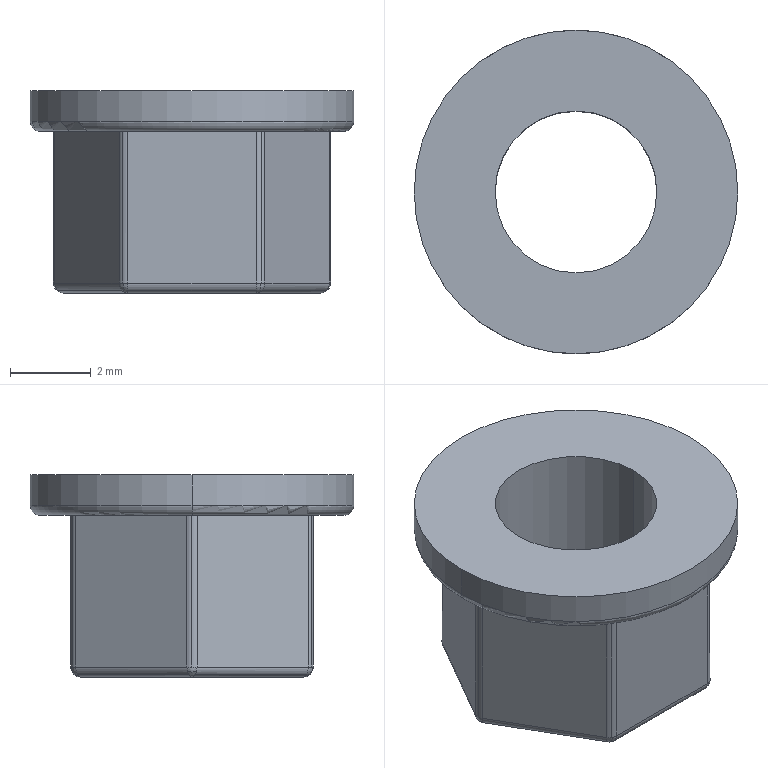Part | SolidWorks | features BaseBody 1 | 1 solid | 53 faces | box 8 x 8 x 5 mm | volume 111.047 mm3 | cylinder 28 | sphere 12 | plane 9 | cone 2 | torus 2 | commonest cylinder face diameters 0.5 x24 4 x2 8 x2
STEP:
#1=CARTESIAN_POINT('',(-2.,0.,0.25));
#2=VERTEX_POINT('',#1);
#3=CARTESIAN_POINT('',(2.,0.,0.25));
#4=VERTEX_POINT('',#3);
#5=CARTESIAN_POINT('',(0.,0.,0.25));
#6=DIRECTION('',(0.,0.,1.));
#7=DIRECTION('',(-1.,0.,0.));
#8=AXIS2_PLACEMENT_3D('',#5,#6,#7);
#9=CIRCLE('',#8,2.);
#10=EDGE_CURVE('',#2,#4,#9,.T.);
#11=ORIENTED_EDGE('',*,*,#10,.T.);
#12=CARTESIAN_POINT('',(2.25,0.,0.));
#13=VERTEX_POINT('',#12);
#14=CARTESIAN_POINT('',(2.125,0.,0.125));
#15=DIRECTION('',(0.7071,0.,-0.7071));
#16=VECTOR('',#15,1000.);
#17=LINE('',#14,#16);
#18=EDGE_CURVE('',#4,#13,#17,.T.);
#19=ORIENTED_EDGE('',*,*,#18,.T.);
#20=CARTESIAN_POINT('',(-2.25,0.,0.));
#21=VERTEX_POINT('',#20);
#22=CARTESIAN_POINT('',(0.,0.,0.));
#23=DIRECTION('',(0.,0.,-1.));
#24=DIRECTION('',(-1.,0.,0.));
#25=AXIS2_PLACEMENT_3D('',#22,#23,#24);
#26=CIRCLE('',#25,2.25);
#27=EDGE_CURVE('',#13,#21,#26,.T.);
#28=ORIENTED_EDGE('',*,*,#27,.T.);
#29=CARTESIAN_POINT('',(-2.125,0.,0.125));
#30=DIRECTION('',(-0.7071,0.,-0.7071));
#31=VECTOR('',#30,1000.);
#32=LINE('',#29,#31);
#33=EDGE_CURVE('',#2,#21,#32,.T.);
#34=ORIENTED_EDGE('',*,*,#33,.F.);
#35=EDGE_LOOP('',(#11,#19,#28,#34));
#36=FACE_OUTER_BOUND('',#35,.T.);
#37=CARTESIAN_POINT('',(0.,0.,0.125));
#38=DIRECTION('',(0.,0.,-1.));
#39=DIRECTION('',(-1.,0.,0.));
#40=AXIS2_PLACEMENT_3D('',#37,#38,#39);
#41=CONICAL_SURFACE('',#40,2.125,0.7854);
#42=ADVANCED_FACE('',(#36),#41,.F.);
#43=CARTESIAN_POINT('',(2.,0.,5.));
#44=VERTEX_POINT('',#43);
#45=CARTESIAN_POINT('',(-2.,0.,5.));
#46=VERTEX_POINT('',#45);
#47=CARTESIAN_POINT('',(0.,0.,5.));
#48=DIRECTION('',(0.,0.,-1.));
#49=DIRECTION('',(-1.,0.,0.));
#50=AXIS2_PLACEMENT_3D('',#47,#48,#49);
#51=CIRCLE('',#50,2.);
#52=EDGE_CURVE('',#44,#46,#51,.T.);
#53=ORIENTED_EDGE('',*,*,#52,.F.);
#54=CARTESIAN_POINT('',(2.,0.,0.));
#55=DIRECTION('',(0.,0.,-1.));
#56=VECTOR('',#55,1000.);
#57=LINE('',#54,#56);
#58=EDGE_CURVE('',#44,#4,#57,.T.);
#59=ORIENTED_EDGE('',*,*,#58,.T.);
#60=ORIENTED_EDGE('',*,*,#10,.F.);
#61=CARTESIAN_POINT('',(-2.,0.,0.));
#62=DIRECTION('',(0.,0.,-1.));
#63=VECTOR('',#62,1000.);
#64=LINE('',#61,#63);
#65=EDGE_CURVE('',#46,#2,#64,.T.);
#66=ORIENTED_EDGE('',*,*,#65,.F.);
#67=EDGE_LOOP('',(#53,#59,#60,#66));
#68=FACE_OUTER_BOUND('',#67,.T.);
#69=CARTESIAN_POINT('',(0.,0.,0.));
#70=DIRECTION('',(0.,0.,-1.));
#71=DIRECTION('',(-1.,0.,0.));
#72=AXIS2_PLACEMENT_3D('',#69,#70,#71);
#73=CYLINDRICAL_SURFACE('',#72,2.);
#74=ADVANCED_FACE('',(#68),#73,.F.);
#75=CARTESIAN_POINT('',(-1.668,-2.796,0.01788));
#76=VERTEX_POINT('',#75);
#77=CARTESIAN_POINT('',(-1.741,-2.838,0.07322));
#78=VERTEX_POINT('',#77);
#79=CARTESIAN_POINT('',(-1.588,-2.75,0.25));
#80=DIRECTION('',(-0.5,0.866,0.));
#81=DIRECTION('',(0.,0.,-1.));
#82=AXIS2_PLACEMENT_3D('',#79,#80,#81);
#83=CIRCLE('',#82,0.25);
#84=EDGE_CURVE('',#76,#78,#83,.T.);
#85=ORIENTED_EDGE('',*,*,#84,.F.);
#86=CARTESIAN_POINT('',(-1.681,-2.982,0.25));
#87=VERTEX_POINT('',#86);
#88=CARTESIAN_POINT('',(-1.588,-2.75,0.25));
#89=DIRECTION('',(-0.9014,0.3603,0.2402));
#90=DIRECTION('',(-0.3712,-0.9286,0.));
#91=AXIS2_PLACEMENT_3D('',#88,#89,#90);
#92=CIRCLE('',#91,0.25);
#93=EDGE_CURVE('',#76,#87,#92,.T.);
#94=ORIENTED_EDGE('',*,*,#93,.T.);
#95=CARTESIAN_POINT('',(-1.713,-2.967,0.25));
#96=VERTEX_POINT('',#95);
#97=CARTESIAN_POINT('',(-1.588,-2.75,0.25));
#98=DIRECTION('',(0.,0.,1.));
#99=DIRECTION('',(-0.866,-0.5,0.));
#100=AXIS2_PLACEMENT_3D('',#97,#98,#99);
#101=CIRCLE('',#100,0.25);
#102=EDGE_CURVE('',#96,#87,#101,.T.);
#103=ORIENTED_EDGE('',*,*,#102,.F.);
#104=CARTESIAN_POINT('',(-1.804,-2.875,0.25));
#105=VERTEX_POINT('',#104);
#106=CARTESIAN_POINT('',(-1.588,-2.75,0.25));
#107=DIRECTION('',(0.,0.,1.));
#108=DIRECTION('',(-0.866,-0.5,0.));
#109=AXIS2_PLACEMENT_3D('',#106,#107,#108);
#110=CIRCLE('',#109,0.25);
#111=EDGE_CURVE('',#105,#96,#110,.T.);
#112=ORIENTED_EDGE('',*,*,#111,.F.);
#113=CARTESIAN_POINT('',(-1.588,-2.75,0.25));
#114=DIRECTION('',(-0.5,0.866,0.));
#115=DIRECTION('',(0.,0.,-1.));
#116=AXIS2_PLACEMENT_3D('',#113,#114,#115);
#117=CIRCLE('',#116,0.25);
#118=EDGE_CURVE('',#78,#105,#117,.T.);
#119=ORIENTED_EDGE('',*,*,#118,.F.);
#120=EDGE_LOOP('',(#85,#94,#103,#112,#119));
#121=FACE_OUTER_BOUND('',#120,.T.);
#122=CARTESIAN_POINT('',(-1.588,-2.75,0.25));
#123=DIRECTION('',(0.9014,-0.3603,-0.2402));
#124=DIRECTION('',(-0.433,-0.75,-0.5));
#125=AXIS2_PLACEMENT_3D('',#122,#123,#124);
#126=SPHERICAL_SURFACE('',#125,0.25);
#127=ADVANCED_FACE('',(#121),#126,.T.);
#128=CARTESIAN_POINT('',(-3.369,-0.1118,0.1382));
#129=VERTEX_POINT('',#128);
#130=CARTESIAN_POINT('',(-3.329,-0.08839,0.07322));
#131=VERTEX_POINT('',#130);
#132=CARTESIAN_POINT('',(-3.175,0.,0.25));
#133=DIRECTION('',(0.5,-0.866,0.));
#134=DIRECTION('',(-0.866,-0.5,0.));
#135=AXIS2_PLACEMENT_3D('',#132,#133,#134);
#136=CIRCLE('',#135,0.25);
#137=EDGE_CURVE('',#129,#131,#136,.T.);
#138=ORIENTED_EDGE('',*,*,#137,.F.);
#139=CARTESIAN_POINT('',(-3.369,0.1118,0.1382));
#140=VERTEX_POINT('',#139);
#141=CARTESIAN_POINT('',(-3.175,0.,0.25));
#142=DIRECTION('',(0.5,0.,-0.866));
#143=DIRECTION('',(-0.866,0.,-0.5));
#144=AXIS2_PLACEMENT_3D('',#141,#142,#143);
#145=CIRCLE('',#144,0.25);
#146=EDGE_CURVE('',#129,#140,#145,.T.);
#147=ORIENTED_EDGE('',*,*,#146,.T.);
#148=CARTESIAN_POINT('',(-3.329,0.08839,0.07322));
#149=VERTEX_POINT('',#148);
#150=CARTESIAN_POINT('',(-3.175,0.,0.25));
#151=DIRECTION('',(0.5,0.866,0.));
#152=DIRECTION('',(0.,0.,-1.));
#153=AXIS2_PLACEMENT_3D('',#150,#151,#152);
#154=CIRCLE('',#153,0.25);
#155=EDGE_CURVE('',#149,#140,#154,.T.);
#156=ORIENTED_EDGE('',*,*,#155,.F.);
#157=CARTESIAN_POINT('',(-3.175,0.,0.));
#158=VERTEX_POINT('',#157);
#159=CARTESIAN_POINT('',(-3.175,0.,0.25));
#160=DIRECTION('',(0.5,0.866,0.));
#161=DIRECTION('',(0.,0.,-1.));
#162=AXIS2_PLACEMENT_3D('',#159,#160,#161);
#163=CIRCLE('',#162,0.25);
#164=EDGE_CURVE('',#158,#149,#163,.T.);
#165=ORIENTED_EDGE('',*,*,#164,.F.);
#166=CARTESIAN_POINT('',(-3.175,0.,0.25));
#167=DIRECTION('',(0.5,-0.866,0.));
#168=DIRECTION('',(-0.866,-0.5,0.));
#169=AXIS2_PLACEMENT_3D('',#166,#167,#168);
#170=CIRCLE('',#169,0.25);
#171=EDGE_CURVE('',#131,#158,#170,.T.);
#172=ORIENTED_EDGE('',*,*,#171,.F.);
#173=EDGE_LOOP('',(#138,#147,#156,#165,#172));
#174=FACE_OUTER_BOUND('',#173,.T.);
#175=CARTESIAN_POINT('',(-3.175,0.,0.25));
#176=DIRECTION('',(-0.5,0.,0.866));
#177=DIRECTION('',(-0.866,0.,-0.5));
#178=AXIS2_PLACEMENT_3D('',#175,#176,#177);
#179=SPHERICAL_SURFACE('',#178,0.25);
#180=ADVANCED_FACE('',(#174),#179,.T.);
#181=CARTESIAN_POINT('',(-3.392,-0.125,0.25));
#182=VERTEX_POINT('',#181);
#183=CARTESIAN_POINT('',(-3.175,0.,0.25));
#184=DIRECTION('',(0.5,-0.866,0.));
#185=DIRECTION('',(-0.866,-0.5,0.));
#186=AXIS2_PLACEMENT_3D('',#183,#184,#185);
#187=CIRCLE('',#186,0.25);
#188=EDGE_CURVE('',#182,#129,#187,.T.);
#189=ORIENTED_EDGE('',*,*,#188,.T.);
#190=ORIENTED_EDGE('',*,*,#137,.T.);
#191=CARTESIAN_POINT('',(-2.968,-0.7134,0.07322));
#192=DIRECTION('',(0.5,-0.866,0.));
#193=VECTOR('',#192,1000.);
#194=LINE('',#191,#193);
#195=EDGE_CURVE('',#131,#78,#194,.T.);
#196=ORIENTED_EDGE('',*,*,#195,.T.);
#197=ORIENTED_EDGE('',*,*,#118,.T.);
#198=CARTESIAN_POINT('',(-3.031,-0.75,0.25));
#199=DIRECTION('',(-0.5,0.866,0.));
#200=VECTOR('',#199,1000.);
#201=LINE('',#198,#200);
#202=EDGE_CURVE('',#105,#182,#201,.T.);
#203=ORIENTED_EDGE('',*,*,#202,.T.);
#204=EDGE_LOOP('',(#189,#190,#196,#197,#203));
#205=FACE_OUTER_BOUND('',#204,.T.);
#206=CARTESIAN_POINT('',(-2.815,-0.625,0.25));
#207=DIRECTION('',(0.5,-0.866,0.));
#208=DIRECTION('',(-0.6124,-0.3536,-0.7071));
#209=AXIS2_PLACEMENT_3D('',#206,#207,#208);
#210=CYLINDRICAL_SURFACE('',#209,0.25);
#211=ADVANCED_FACE('',(#205),#210,.T.);
#212=CARTESIAN_POINT('',(-3.392,-0.125,4.));
#213=VERTEX_POINT('',#212);
#214=CARTESIAN_POINT('',(-3.425,0.,4.));
#215=VERTEX_POINT('',#214);
#216=CARTESIAN_POINT('',(-3.175,0.,4.));
#217=DIRECTION('',(0.,0.,-1.));
#218=DIRECTION('',(-1.,0.,0.));
#219=AXIS2_PLACEMENT_3D('',#216,#217,#218);
#220=CIRCLE('',#219,0.25);
#221=EDGE_CURVE('',#213,#215,#220,.T.);
#222=ORIENTED_EDGE('',*,*,#221,.T.);
#223=CARTESIAN_POINT('',(-3.425,0.,0.25));
#224=VERTEX_POINT('',#223);
#225=CARTESIAN_POINT('',(-3.425,0.,0.));
#226=DIRECTION('',(0.,0.,-1.));
#227=VECTOR('',#226,1000.);
#228=LINE('',#225,#227);
#229=EDGE_CURVE('',#215,#224,#228,.T.);
#230=ORIENTED_EDGE('',*,*,#229,.T.);
#231=CARTESIAN_POINT('',(-3.175,0.,0.25));
#232=DIRECTION('',(0.,0.,1.));
#233=DIRECTION('',(-0.866,0.5,0.));
#234=AXIS2_PLACEMENT_3D('',#231,#232,#233);
#235=CIRCLE('',#234,0.25);
#236=EDGE_CURVE('',#224,#182,#235,.T.);
#237=ORIENTED_EDGE('',*,*,#236,.T.);
#238=CARTESIAN_POINT('',(-3.392,-0.125,0.));
#239=DIRECTION('',(0.,0.,1.));
#240=VECTOR('',#239,1000.);
#241=LINE('',#238,#240);
#242=EDGE_CURVE('',#182,#213,#241,.T.);
#243=ORIENTED_EDGE('',*,*,#242,.T.);
#244=EDGE_LOOP('',(#222,#230,#237,#243));
#245=FACE_OUTER_BOUND('',#244,.T.);
#246=CARTESIAN_POINT('',(-3.175,0.,0.));
#247=DIRECTION('',(0.,0.,-1.));
#248=DIRECTION('',(-1.,0.,0.));
#249=AXIS2_PLACEMENT_3D('',#246,#247,#248);
#250=CYLINDRICAL_SURFACE('',#249,0.25);
#251=ADVANCED_FACE('',(#245),#250,.T.);
#252=CARTESIAN_POINT('',(1.668,-2.796,0.01788));
#253=VERTEX_POINT('',#252);
#254=CARTESIAN_POINT('',(1.588,-2.75,0.));
#255=VERTEX_POINT('',#254);
#256=CARTESIAN_POINT('',(1.588,-2.75,0.25));
#257=DIRECTION('',(0.5,0.866,0.));
#258=DIRECTION('',(0.866,-0.5,0.));
#259=AXIS2_PLACEMENT_3D('',#256,#257,#258);
#260=CIRCLE('',#259,0.25);
#261=EDGE_CURVE('',#253,#255,#260,.T.);
#262=ORIENTED_EDGE('',*,*,#261,.F.);
#263=CARTESIAN_POINT('',(1.681,-2.982,0.25));
#264=VERTEX_POINT('',#263);
#265=CARTESIAN_POINT('',(1.588,-2.75,0.25));
#266=DIRECTION('',(-0.9014,-0.3603,-0.2402));
#267=DIRECTION('',(0.3712,-0.9286,0.));
#268=AXIS2_PLACEMENT_3D('',#265,#266,#267);
#269=CIRCLE('',#268,0.25);
#270=EDGE_CURVE('',#253,#264,#269,.T.);
#271=ORIENTED_EDGE('',*,*,#270,.T.);
#272=CARTESIAN_POINT('',(1.588,-3.,0.25));
#273=VERTEX_POINT('',#272);
#274=CARTESIAN_POINT('',(1.588,-2.75,0.25));
#275=DIRECTION('',(0.,0.,1.));
#276=DIRECTION('',(0.,-1.,0.));
#277=AXIS2_PLACEMENT_3D('',#274,#275,#276);
#278=CIRCLE('',#277,0.25);
#279=EDGE_CURVE('',#273,#264,#278,.T.);
#280=ORIENTED_EDGE('',*,*,#279,.F.);
#281=CARTESIAN_POINT('',(1.588,-2.927,0.07322));
#282=VERTEX_POINT('',#281);
#283=CARTESIAN_POINT('',(1.588,-2.75,0.25));
#284=DIRECTION('',(-1.,0.,0.));
#285=DIRECTION('',(0.,0.,-1.));
#286=AXIS2_PLACEMENT_3D('',#283,#284,#285);
#287=CIRCLE('',#286,0.25);
#288=EDGE_CURVE('',#282,#273,#287,.T.);
#289=ORIENTED_EDGE('',*,*,#288,.F.);
#290=CARTESIAN_POINT('',(1.588,-2.75,0.25));
#291=DIRECTION('',(-1.,0.,0.));
#292=DIRECTION('',(0.,0.,-1.));
#293=AXIS2_PLACEMENT_3D('',#290,#291,#292);
#294=CIRCLE('',#293,0.25);
#295=EDGE_CURVE('',#255,#282,#294,.T.);
#296=ORIENTED_EDGE('',*,*,#295,.F.);
#297=EDGE_LOOP('',(#262,#271,#280,#289,#296));
#298=FACE_OUTER_BOUND('',#297,.T.);
#299=CARTESIAN_POINT('',(1.588,-2.75,0.25));
#300=DIRECTION('',(0.9014,0.3603,0.2402));
#301=DIRECTION('',(0.433,-0.75,-0.5));
#302=AXIS2_PLACEMENT_3D('',#299,#300,#301);
#303=SPHERICAL_SURFACE('',#302,0.25);
#304=ADVANCED_FACE('',(#298),#303,.T.);
#305=CARTESIAN_POINT('',(-1.588,-3.,0.25));
#306=VERTEX_POINT('',#305);
#307=CARTESIAN_POINT('',(-1.588,-2.927,0.07322));
#308=VERTEX_POINT('',#307);
#309=CARTESIAN_POINT('',(-1.588,-2.75,0.25));
#310=DIRECTION('',(1.,0.,0.));
#311=DIRECTION('',(0.,-1.,0.));
#312=AXIS2_PLACEMENT_3D('',#309,#310,#311);
#313=CIRCLE('',#312,0.25);
#314=EDGE_CURVE('',#306,#308,#313,.T.);
#315=ORIENTED_EDGE('',*,*,#314,.T.);
#316=CARTESIAN_POINT('',(-0.866,-2.927,0.07322));
#317=DIRECTION('',(1.,0.,0.));
#318=VECTOR('',#317,1000.);
#319=LINE('',#316,#318);
#320=EDGE_CURVE('',#308,#282,#319,.T.);
#321=ORIENTED_EDGE('',*,*,#320,.T.);
#322=ORIENTED_EDGE('',*,*,#288,.T.);
#323=CARTESIAN_POINT('',(-0.866,-3.,0.25));
#324=DIRECTION('',(-1.,0.,0.));
#325=VECTOR('',#324,1000.);
#326=LINE('',#323,#325);
#327=EDGE_CURVE('',#273,#306,#326,.T.);
#328=ORIENTED_EDGE('',*,*,#327,.T.);
#329=EDGE_LOOP('',(#315,#321,#322,#328));
#330=FACE_OUTER_BOUND('',#329,.T.);
#331=CARTESIAN_POINT('',(-0.866,-2.75,0.25));
#332=DIRECTION('',(1.,0.,0.));
#333=DIRECTION('',(0.,-0.7071,-0.7071));
#334=AXIS2_PLACEMENT_3D('',#331,#332,#333);
#335=CYLINDRICAL_SURFACE('',#334,0.25);
#336=ADVANCED_FACE('',(#330),#335,.T.);
#337=CARTESIAN_POINT('',(-1.681,2.982,0.25));
#338=VERTEX_POINT('',#337);
#339=CARTESIAN_POINT('',(-1.713,2.967,0.25));
#340=VERTEX_POINT('',#339);
#341=CARTESIAN_POINT('',(-1.588,2.75,0.25));
#342=DIRECTION('',(0.,0.,1.));
#343=DIRECTION('',(0.,1.,0.));
#344=AXIS2_PLACEMENT_3D('',#341,#342,#343);
#345=CIRCLE('',#344,0.25);
#346=EDGE_CURVE('',#338,#340,#345,.T.);
#347=ORIENTED_EDGE('',*,*,#346,.F.);
#348=CARTESIAN_POINT('',(-1.668,2.796,0.01788));
#349=VERTEX_POINT('',#348);
#350=CARTESIAN_POINT('',(-1.588,2.75,0.25));
#351=DIRECTION('',(-0.9014,-0.3603,0.2402));
#352=DIRECTION('',(0.3712,-0.9286,0.));
#353=AXIS2_PLACEMENT_3D('',#350,#351,#352);
#354=CIRCLE('',#353,0.25);
#355=EDGE_CURVE('',#338,#349,#354,.T.);
#356=ORIENTED_EDGE('',*,*,#355,.T.);
#357=CARTESIAN_POINT('',(-1.741,2.838,0.07322));
#358=VERTEX_POINT('',#357);
#359=CARTESIAN_POINT('',(-1.588,2.75,0.25));
#360=DIRECTION('',(-0.5,-0.866,0.));
#361=DIRECTION('',(-0.866,0.5,0.));
#362=AXIS2_PLACEMENT_3D('',#359,#360,#361);
#363=CIRCLE('',#362,0.25);
#364=EDGE_CURVE('',#358,#349,#363,.T.);
#365=ORIENTED_EDGE('',*,*,#364,.F.);
#366=CARTESIAN_POINT('',(-1.804,2.875,0.25));
#367=VERTEX_POINT('',#366);
#368=CARTESIAN_POINT('',(-1.588,2.75,0.25));
#369=DIRECTION('',(-0.5,-0.866,0.));
#370=DIRECTION('',(-0.866,0.5,0.));
#371=AXIS2_PLACEMENT_3D('',#368,#369,#370);
#372=CIRCLE('',#371,0.25);
#373=EDGE_CURVE('',#367,#358,#372,.T.);
#374=ORIENTED_EDGE('',*,*,#373,.F.);
#375=CARTESIAN_POINT('',(-1.588,2.75,0.25));
#376=DIRECTION('',(0.,0.,1.));
#377=DIRECTION('',(0.,1.,0.));
#378=AXIS2_PLACEMENT_3D('',#375,#376,#377);
#379=CIRCLE('',#378,0.25);
#380=EDGE_CURVE('',#340,#367,#379,.T.);
#381=ORIENTED_EDGE('',*,*,#380,.F.);
#382=EDGE_LOOP('',(#347,#356,#365,#374,#381));
#383=FACE_OUTER_BOUND('',#382,.T.);
#384=CARTESIAN_POINT('',(-1.588,2.75,0.25));
#385=DIRECTION('',(0.9014,0.3603,-0.2402));
#386=DIRECTION('',(-0.433,0.75,-0.5));
#387=AXIS2_PLACEMENT_3D('',#384,#385,#386);
#388=SPHERICAL_SURFACE('',#387,0.25);
#389=ADVANCED_FACE('',(#383),#388,.T.);
#390=ORIENTED_EDGE('',*,*,#373,.T.);
#391=CARTESIAN_POINT('',(-2.102,2.213,0.07322));
#392=DIRECTION('',(-0.5,-0.866,0.));
#393=VECTOR('',#392,1000.);
#394=LINE('',#391,#393);
#395=EDGE_CURVE('',#358,#149,#394,.T.);
#396=ORIENTED_EDGE('',*,*,#395,.T.);
#397=ORIENTED_EDGE('',*,*,#155,.T.);
#398=CARTESIAN_POINT('',(-3.392,0.125,0.25));
#399=VERTEX_POINT('',#398);
#400=CARTESIAN_POINT('',(-3.175,0.,0.25));
#401=DIRECTION('',(0.5,0.866,0.));
#402=DIRECTION('',(0.,0.,-1.));
#403=AXIS2_PLACEMENT_3D('',#400,#401,#402);
#404=CIRCLE('',#403,0.25);
#405=EDGE_CURVE('',#140,#399,#404,.T.);
#406=ORIENTED_EDGE('',*,*,#405,.T.);
#407=CARTESIAN_POINT('',(-2.165,2.25,0.25));
#408=DIRECTION('',(0.5,0.866,0.));
#409=VECTOR('',#408,1000.);
#410=LINE('',#407,#409);
#411=EDGE_CURVE('',#399,#367,#410,.T.);
#412=ORIENTED_EDGE('',*,*,#411,.T.);
#413=EDGE_LOOP('',(#390,#396,#397,#406,#412));
#414=FACE_OUTER_BOUND('',#413,.T.);
#415=CARTESIAN_POINT('',(-1.949,2.125,0.25));
#416=DIRECTION('',(-0.5,-0.866,0.));
#417=DIRECTION('',(-0.6124,0.3536,-0.7071));
#418=AXIS2_PLACEMENT_3D('',#415,#416,#417);
#419=CYLINDRICAL_SURFACE('',#418,0.25);
#420=ADVANCED_FACE('',(#414),#419,.T.);
#421=CARTESIAN_POINT('',(-1.804,2.875,4.));
#422=VERTEX_POINT('',#421);
#423=CARTESIAN_POINT('',(-1.713,2.967,4.));
#424=VERTEX_POINT('',#423);
#425=CARTESIAN_POINT('',(-1.588,2.75,4.));
#426=DIRECTION('',(0.,0.,-1.));
#427=DIRECTION('',(-0.5,0.866,0.));
#428=AXIS2_PLACEMENT_3D('',#425,#426,#427);
#429=CIRCLE('',#428,0.25);
#430=EDGE_CURVE('',#422,#424,#429,.T.);
#431=ORIENTED_EDGE('',*,*,#430,.T.);
#432=CARTESIAN_POINT('',(-1.713,2.967,0.));
#433=DIRECTION('',(0.,0.,-1.));
#434=VECTOR('',#433,1000.);
#435=LINE('',#432,#434);
#436=EDGE_CURVE('',#424,#340,#435,.T.);
#437=ORIENTED_EDGE('',*,*,#436,.T.);
#438=ORIENTED_EDGE('',*,*,#380,.T.);
#439=CARTESIAN_POINT('',(-1.804,2.875,0.));
#440=DIRECTION('',(0.,0.,1.));
#441=VECTOR('',#440,1000.);
#442=LINE('',#439,#441);
#443=EDGE_CURVE('',#367,#422,#442,.T.);
#444=ORIENTED_EDGE('',*,*,#443,.T.);
#445=EDGE_LOOP('',(#431,#437,#438,#444));
#446=FACE_OUTER_BOUND('',#445,.T.);
#447=CARTESIAN_POINT('',(-1.588,2.75,0.));
#448=DIRECTION('',(0.,0.,-1.));
#449=DIRECTION('',(-0.5,0.866,0.));
#450=AXIS2_PLACEMENT_3D('',#447,#448,#449);
#451=CYLINDRICAL_SURFACE('',#450,0.25);
#452=ADVANCED_FACE('',(#446),#451,.T.);
#453=CARTESIAN_POINT('',(3.369,0.1118,0.1382));
#454=VERTEX_POINT('',#453);
#455=CARTESIAN_POINT('',(3.329,0.08839,0.07322));
#456=VERTEX_POINT('',#455);
#457=CARTESIAN_POINT('',(3.175,0.,0.25));
#458=DIRECTION('',(-0.5,0.866,0.));
#459=DIRECTION('',(0.866,0.5,0.));
#460=AXIS2_PLACEMENT_3D('',#457,#458,#459);
#461=CIRCLE('',#460,0.25);
#462=EDGE_CURVE('',#454,#456,#461,.T.);
#463=ORIENTED_EDGE('',*,*,#462,.F.);
#464=CARTESIAN_POINT('',(3.369,-0.1118,0.1382));
#465=VERTEX_POINT('',#464);
#466=CARTESIAN_POINT('',(3.175,0.,0.25));
#467=DIRECTION('',(-0.5,0.,-0.866));
#468=DIRECTION('',(-0.866,0.,0.5));
#469=AXIS2_PLACEMENT_3D('',#466,#467,#468);
#470=CIRCLE('',#469,0.25);
#471=EDGE_CURVE('',#454,#465,#470,.T.);
#472=ORIENTED_EDGE('',*,*,#471,.T.);
#473=CARTESIAN_POINT('',(3.329,-0.08839,0.07322));
#474=VERTEX_POINT('',#473);
#475=CARTESIAN_POINT('',(3.175,0.,0.25));
#476=DIRECTION('',(-0.5,-0.866,0.));
#477=DIRECTION('',(0.,0.,-1.));
#478=AXIS2_PLACEMENT_3D('',#475,#476,#477);
#479=CIRCLE('',#478,0.25);
#480=EDGE_CURVE('',#474,#465,#479,.T.);
#481=ORIENTED_EDGE('',*,*,#480,.F.);
#482=CARTESIAN_POINT('',(3.175,0.,0.));
#483=VERTEX_POINT('',#482);
#484=CARTESIAN_POINT('',(3.175,0.,0.25));
#485=DIRECTION('',(-0.5,-0.866,0.));
#486=DIRECTION('',(0.,0.,-1.));
#487=AXIS2_PLACEMENT_3D('',#484,#485,#486);
#488=CIRCLE('',#487,0.25);
#489=EDGE_CURVE('',#483,#474,#488,.T.);
#490=ORIENTED_EDGE('',*,*,#489,.F.);
#491=CARTESIAN_POINT('',(3.175,0.,0.25));
#492=DIRECTION('',(-0.5,0.866,0.));
#493=DIRECTION('',(0.866,0.5,0.));
#494=AXIS2_PLACEMENT_3D('',#491,#492,#493);
#495=CIRCLE('',#494,0.25);
#496=EDGE_CURVE('',#456,#483,#495,.T.);
#497=ORIENTED_EDGE('',*,*,#496,.F.);
#498=EDGE_LOOP('',(#463,#472,#481,#490,#497));
#499=FACE_OUTER_BOUND('',#498,.T.);
#500=CARTESIAN_POINT('',(3.175,0.,0.25));
#501=DIRECTION('',(0.5,0.,0.866));
#502=DIRECTION('',(0.866,0.,-0.5));
#503=AXIS2_PLACEMENT_3D('',#500,#501,#502);
#504=SPHERICAL_SURFACE('',#503,0.25);
#505=ADVANCED_FACE('',(#499),#504,.T.);
#506=CARTESIAN_POINT('',(1.681,2.982,0.25));
#507=VERTEX_POINT('',#506);
#508=CARTESIAN_POINT('',(1.588,3.,0.25));
#509=VERTEX_POINT('',#508);
#510=CARTESIAN_POINT('',(1.588,2.75,0.25));
#511=DIRECTION('',(0.,0.,1.));
#512=DIRECTION('',(0.866,0.5,0.));
#513=AXIS2_PLACEMENT_3D('',#510,#511,#512);
#514=CIRCLE('',#513,0.25);
#515=EDGE_CURVE('',#507,#509,#514,.T.);
#516=ORIENTED_EDGE('',*,*,#515,.F.);
#517=CARTESIAN_POINT('',(1.668,2.796,0.01788));
#518=VERTEX_POINT('',#517);
#519=CARTESIAN_POINT('',(1.588,2.75,0.25));
#520=DIRECTION('',(-0.9014,0.3603,-0.2402));
#521=DIRECTION('',(-0.3712,-0.9286,0.));
#522=AXIS2_PLACEMENT_3D('',#519,#520,#521);
#523=CIRCLE('',#522,0.25);
#524=EDGE_CURVE('',#507,#518,#523,.T.);
#525=ORIENTED_EDGE('',*,*,#524,.T.);
#526=CARTESIAN_POINT('',(1.588,2.75,0.));
#527=VERTEX_POINT('',#526);
#528=CARTESIAN_POINT('',(1.588,2.75,0.25));
#529=DIRECTION('',(0.5,-0.866,0.));
#530=DIRECTION('',(0.,0.,-1.));
#531=AXIS2_PLACEMENT_3D('',#528,#529,#530);
#532=CIRCLE('',#531,0.25);
#533=EDGE_CURVE('',#527,#518,#532,.T.);
#534=ORIENTED_EDGE('',*,*,#533,.F.);
#535=CARTESIAN_POINT('',(1.588,2.927,0.07322));
#536=VERTEX_POINT('',#535);
#537=CARTESIAN_POINT('',(1.588,2.75,0.25));
#538=DIRECTION('',(-1.,0.,0.));
#539=DIRECTION('',(0.,1.,0.));
#540=AXIS2_PLACEMENT_3D('',#537,#538,#539);
#541=CIRCLE('',#540,0.25);
#542=EDGE_CURVE('',#536,#527,#541,.T.);
#543=ORIENTED_EDGE('',*,*,#542,.F.);
#544=CARTESIAN_POINT('',(1.588,2.75,0.25));
#545=DIRECTION('',(-1.,0.,0.));
#546=DIRECTION('',(0.,1.,0.));
#547=AXIS2_PLACEMENT_3D('',#544,#545,#546);
#548=CIRCLE('',#547,0.25);
#549=EDGE_CURVE('',#509,#536,#548,.T.);
#550=ORIENTED_EDGE('',*,*,#549,.F.);
#551=EDGE_LOOP('',(#516,#525,#534,#543,#550));
#552=FACE_OUTER_BOUND('',#551,.T.);
#553=CARTESIAN_POINT('',(1.588,2.75,0.25));
#554=DIRECTION('',(0.9014,-0.3603,0.2402));
#555=DIRECTION('',(0.433,0.75,-0.5));
#556=AXIS2_PLACEMENT_3D('',#553,#554,#555);
#557=SPHERICAL_SURFACE('',#556,0.25);
#558=ADVANCED_FACE('',(#552),#557,.T.);
#559=ORIENTED_EDGE('',*,*,#549,.T.);
#560=CARTESIAN_POINT('',(-1.588,2.927,0.07322));
#561=VERTEX_POINT('',#560);
#562=CARTESIAN_POINT('',(0.866,2.927,0.07322));
#563=DIRECTION('',(-1.,0.,0.));
#564=VECTOR('',#563,1000.);
#565=LINE('',#562,#564);
#566=EDGE_CURVE('',#536,#561,#565,.T.);
#567=ORIENTED_EDGE('',*,*,#566,.T.);
#568=CARTESIAN_POINT('',(-1.588,3.,0.25));
#569=VERTEX_POINT('',#568);
#570=CARTESIAN_POINT('',(-1.588,2.75,0.25));
#571=DIRECTION('',(1.,0.,0.));
#572=DIRECTION('',(0.,0.,-1.));
#573=AXIS2_PLACEMENT_3D('',#570,#571,#572);
#574=CIRCLE('',#573,0.25);
#575=EDGE_CURVE('',#561,#569,#574,.T.);
#576=ORIENTED_EDGE('',*,*,#575,.T.);
#577=CARTESIAN_POINT('',(0.866,3.,0.25));
#578=DIRECTION('',(1.,0.,0.));
#579=VECTOR('',#578,1000.);
#580=LINE('',#577,#579);
#581=EDGE_CURVE('',#569,#509,#580,.T.);
#582=ORIENTED_EDGE('',*,*,#581,.T.);
#583=EDGE_LOOP('',(#559,#567,#576,#582));
#584=FACE_OUTER_BOUND('',#583,.T.);
#585=CARTESIAN_POINT('',(0.866,2.75,0.25));
#586=DIRECTION('',(-1.,0.,0.));
#587=DIRECTION('',(0.,0.7071,-0.7071));
#588=AXIS2_PLACEMENT_3D('',#585,#586,#587);
#589=CYLINDRICAL_SURFACE('',#588,0.25);
#590=ADVANCED_FACE('',(#584),#589,.T.);
#591=CARTESIAN_POINT('',(1.588,3.,4.));
#592=VERTEX_POINT('',#591);
#593=CARTESIAN_POINT('',(1.713,2.967,4.));
#594=VERTEX_POINT('',#593);
#595=CARTESIAN_POINT('',(1.588,2.75,4.));
#596=DIRECTION('',(0.,0.,-1.));
#597=DIRECTION('',(0.5,0.866,0.));
#598=AXIS2_PLACEMENT_3D('',#595,#596,#597);
#599=CIRCLE('',#598,0.25);
#600=EDGE_CURVE('',#592,#594,#599,.T.);
#601=ORIENTED_EDGE('',*,*,#600,.T.);
#602=CARTESIAN_POINT('',(1.713,2.967,0.25));
#603=VERTEX_POINT('',#602);
#604=CARTESIAN_POINT('',(1.713,2.967,0.));
#605=DIRECTION('',(0.,0.,-1.));
#606=VECTOR('',#605,1000.);
#607=LINE('',#604,#606);
#608=EDGE_CURVE('',#594,#603,#607,.T.);
#609=ORIENTED_EDGE('',*,*,#608,.T.);
#610=CARTESIAN_POINT('',(1.588,2.75,0.25));
#611=DIRECTION('',(0.,0.,1.));
#612=DIRECTION('',(0.866,0.5,0.));
#613=AXIS2_PLACEMENT_3D('',#610,#611,#612);
#614=CIRCLE('',#613,0.25);
#615=EDGE_CURVE('',#603,#507,#614,.T.);
#616=ORIENTED_EDGE('',*,*,#615,.T.);
#617=ORIENTED_EDGE('',*,*,#515,.T.);
#618=CARTESIAN_POINT('',(1.588,3.,0.));
#619=DIRECTION('',(0.,0.,1.));
#620=VECTOR('',#619,1000.);
#621=LINE('',#618,#620);
#622=EDGE_CURVE('',#509,#592,#621,.T.);
#623=ORIENTED_EDGE('',*,*,#622,.T.);
#624=EDGE_LOOP('',(#601,#609,#616,#617,#623));
#625=FACE_OUTER_BOUND('',#624,.T.);
#626=CARTESIAN_POINT('',(1.588,2.75,0.));
#627=DIRECTION('',(0.,0.,-1.));
#628=DIRECTION('',(0.5,0.866,0.));
#629=AXIS2_PLACEMENT_3D('',#626,#627,#628);
#630=CYLINDRICAL_SURFACE('',#629,0.25);
#631=ADVANCED_FACE('',(#625),#630,.T.);
#632=CARTESIAN_POINT('',(3.392,0.125,0.25));
#633=VERTEX_POINT('',#632);
#634=CARTESIAN_POINT('',(3.175,0.,0.25));
#635=DIRECTION('',(-0.5,0.866,0.));
#636=DIRECTION('',(0.866,0.5,0.));
#637=AXIS2_PLACEMENT_3D('',#634,#635,#636);
#638=CIRCLE('',#637,0.25);
#639=EDGE_CURVE('',#633,#454,#638,.T.);
#640=ORIENTED_EDGE('',*,*,#639,.T.);
#641=ORIENTED_EDGE('',*,*,#462,.T.);
#642=CARTESIAN_POINT('',(1.741,2.838,0.07322));
#643=VERTEX_POINT('',#642);
#644=CARTESIAN_POINT('',(2.968,0.7134,0.07322));
#645=DIRECTION('',(-0.5,0.866,0.));
#646=VECTOR('',#645,1000.);
#647=LINE('',#644,#646);
#648=EDGE_CURVE('',#456,#643,#647,.T.);
#649=ORIENTED_EDGE('',*,*,#648,.T.);
#650=CARTESIAN_POINT('',(1.804,2.875,0.25));
#651=VERTEX_POINT('',#650);
#652=CARTESIAN_POINT('',(1.588,2.75,0.25));
#653=DIRECTION('',(0.5,-0.866,0.));
#654=DIRECTION('',(0.,0.,-1.));
#655=AXIS2_PLACEMENT_3D('',#652,#653,#654);
#656=CIRCLE('',#655,0.25);
#657=EDGE_CURVE('',#643,#651,#656,.T.);
#658=ORIENTED_EDGE('',*,*,#657,.T.);
#659=CARTESIAN_POINT('',(3.031,0.75,0.25));
#660=DIRECTION('',(0.5,-0.866,0.));
#661=VECTOR('',#660,1000.);
#662=LINE('',#659,#661);
#663=EDGE_CURVE('',#651,#633,#662,.T.);
#664=ORIENTED_EDGE('',*,*,#663,.T.);
#665=EDGE_LOOP('',(#640,#641,#649,#658,#664));
#666=FACE_OUTER_BOUND('',#665,.T.);
#667=CARTESIAN_POINT('',(2.815,0.625,0.25));
#668=DIRECTION('',(-0.5,0.866,0.));
#669=DIRECTION('',(0.6124,0.3536,-0.7071));
#670=AXIS2_PLACEMENT_3D('',#667,#668,#669);
#671=CYLINDRICAL_SURFACE('',#670,0.25);
#672=ADVANCED_FACE('',(#666),#671,.T.);
#673=CARTESIAN_POINT('',(3.392,0.125,4.));
#674=VERTEX_POINT('',#673);
#675=CARTESIAN_POINT('',(3.425,0.,4.));
#676=VERTEX_POINT('',#675);
#677=CARTESIAN_POINT('',(3.175,0.,4.));
#678=DIRECTION('',(0.,0.,-1.));
#679=DIRECTION('',(1.,0.,0.));
#680=AXIS2_PLACEMENT_3D('',#677,#678,#679);
#681=CIRCLE('',#680,0.25);
#682=EDGE_CURVE('',#674,#676,#681,.T.);
#683=ORIENTED_EDGE('',*,*,#682,.T.);
#684=CARTESIAN_POINT('',(3.425,0.,0.25));
#685=VERTEX_POINT('',#684);
#686=CARTESIAN_POINT('',(3.425,0.,0.));
#687=DIRECTION('',(0.,0.,-1.));
#688=VECTOR('',#687,1000.);
#689=LINE('',#686,#688);
#690=EDGE_CURVE('',#676,#685,#689,.T.);
#691=ORIENTED_EDGE('',*,*,#690,.T.);
#692=CARTESIAN_POINT('',(3.175,0.,0.25));
#693=DIRECTION('',(0.,0.,1.));
#694=DIRECTION('',(0.866,-0.5,0.));
#695=AXIS2_PLACEMENT_3D('',#692,#693,#694);
#696=CIRCLE('',#695,0.25);
#697=EDGE_CURVE('',#685,#633,#696,.T.);
#698=ORIENTED_EDGE('',*,*,#697,.T.);
#699=CARTESIAN_POINT('',(3.392,0.125,0.));
#700=DIRECTION('',(0.,0.,1.));
#701=VECTOR('',#700,1000.);
#702=LINE('',#699,#701);
#703=EDGE_CURVE('',#633,#674,#702,.T.);
#704=ORIENTED_EDGE('',*,*,#703,.T.);
#705=EDGE_LOOP('',(#683,#691,#698,#704));
#706=FACE_OUTER_BOUND('',#705,.T.);
#707=CARTESIAN_POINT('',(3.175,0.,0.));
#708=DIRECTION('',(0.,0.,-1.));
#709=DIRECTION('',(1.,0.,0.));
#710=AXIS2_PLACEMENT_3D('',#707,#708,#709);
#711=CYLINDRICAL_SURFACE('',#710,0.25);
#712=ADVANCED_FACE('',(#706),#711,.T.);
#713=CARTESIAN_POINT('',(1.804,-2.875,0.25));
#714=VERTEX_POINT('',#713);
#715=CARTESIAN_POINT('',(1.741,-2.838,0.07322));
#716=VERTEX_POINT('',#715);
#717=CARTESIAN_POINT('',(1.588,-2.75,0.25));
#718=DIRECTION('',(0.5,0.866,0.));
#719=DIRECTION('',(0.866,-0.5,0.));
#720=AXIS2_PLACEMENT_3D('',#717,#718,#719);
#721=CIRCLE('',#720,0.25);
#722=EDGE_CURVE('',#714,#716,#721,.T.);
#723=ORIENTED_EDGE('',*,*,#722,.T.);
#724=CARTESIAN_POINT('',(2.102,-2.213,0.07322));
#725=DIRECTION('',(0.5,0.866,0.));
#726=VECTOR('',#725,1000.);
#727=LINE('',#724,#726);
#728=EDGE_CURVE('',#716,#474,#727,.T.);
#729=ORIENTED_EDGE('',*,*,#728,.T.);
#730=ORIENTED_EDGE('',*,*,#480,.T.);
#731=CARTESIAN_POINT('',(3.392,-0.125,0.25));
#732=VERTEX_POINT('',#731);
#733=CARTESIAN_POINT('',(3.175,0.,0.25));
#734=DIRECTION('',(-0.5,-0.866,0.));
#735=DIRECTION('',(0.,0.,-1.));
#736=AXIS2_PLACEMENT_3D('',#733,#734,#735);
#737=CIRCLE('',#736,0.25);
#738=EDGE_CURVE('',#465,#732,#737,.T.);
#739=ORIENTED_EDGE('',*,*,#738,.T.);
#740=CARTESIAN_POINT('',(2.165,-2.25,0.25));
#741=DIRECTION('',(-0.5,-0.866,0.));
#742=VECTOR('',#741,1000.);
#743=LINE('',#740,#742);
#744=EDGE_CURVE('',#732,#714,#743,.T.);
#745=ORIENTED_EDGE('',*,*,#744,.T.);
#746=EDGE_LOOP('',(#723,#729,#730,#739,#745));
#747=FACE_OUTER_BOUND('',#746,.T.);
#748=CARTESIAN_POINT('',(1.949,-2.125,0.25));
#749=DIRECTION('',(0.5,0.866,0.));
#750=DIRECTION('',(0.6124,-0.3536,-0.7071));
#751=AXIS2_PLACEMENT_3D('',#748,#749,#750);
#752=CYLINDRICAL_SURFACE('',#751,0.25);
#753=ADVANCED_FACE('',(#747),#752,.T.);
#754=CARTESIAN_POINT('',(1.804,-2.875,4.));
#755=VERTEX_POINT('',#754);
#756=CARTESIAN_POINT('',(1.713,-2.967,4.));
#757=VERTEX_POINT('',#756);
#758=CARTESIAN_POINT('',(1.588,-2.75,4.));
#759=DIRECTION('',(0.,0.,-1.));
#760=DIRECTION('',(0.5,-0.866,0.));
#761=AXIS2_PLACEMENT_3D('',#758,#759,#760);
#762=CIRCLE('',#761,0.25);
#763=EDGE_CURVE('',#755,#757,#762,.T.);
#764=ORIENTED_EDGE('',*,*,#763,.T.);
#765=CARTESIAN_POINT('',(1.713,-2.967,0.25));
#766=VERTEX_POINT('',#765);
#767=CARTESIAN_POINT('',(1.713,-2.967,0.));
#768=DIRECTION('',(0.,0.,-1.));
#769=VECTOR('',#768,1000.);
#770=LINE('',#767,#769);
#771=EDGE_CURVE('',#757,#766,#770,.T.);
#772=ORIENTED_EDGE('',*,*,#771,.T.);
#773=CARTESIAN_POINT('',(1.588,-2.75,0.25));
#774=DIRECTION('',(0.,0.,1.));
#775=DIRECTION('',(0.,-1.,0.));
#776=AXIS2_PLACEMENT_3D('',#773,#774,#775);
#777=CIRCLE('',#776,0.25);
#778=EDGE_CURVE('',#766,#714,#777,.T.);
#779=ORIENTED_EDGE('',*,*,#778,.T.);
#780=CARTESIAN_POINT('',(1.804,-2.875,0.));
#781=DIRECTION('',(0.,0.,1.));
#782=VECTOR('',#781,1000.);
#783=LINE('',#780,#782);
#784=EDGE_CURVE('',#714,#755,#783,.T.);
#785=ORIENTED_EDGE('',*,*,#784,.T.);
#786=EDGE_LOOP('',(#764,#772,#779,#785));
#787=FACE_OUTER_BOUND('',#786,.T.);
#788=CARTESIAN_POINT('',(1.588,-2.75,0.));
#789=DIRECTION('',(0.,0.,-1.));
#790=DIRECTION('',(0.5,-0.866,0.));
#791=AXIS2_PLACEMENT_3D('',#788,#789,#790);
#792=CYLINDRICAL_SURFACE('',#791,0.25);
#793=ADVANCED_FACE('',(#787),#792,.T.);
#794=CARTESIAN_POINT('',(-1.588,-3.,4.));
#795=VERTEX_POINT('',#794);
#796=CARTESIAN_POINT('',(-1.713,-2.967,4.));
#797=VERTEX_POINT('',#796);
#798=CARTESIAN_POINT('',(-1.588,-2.75,4.));
#799=DIRECTION('',(0.,0.,-1.));
#800=DIRECTION('',(-0.5,-0.866,0.));
#801=AXIS2_PLACEMENT_3D('',#798,#799,#800);
#802=CIRCLE('',#801,0.25);
#803=EDGE_CURVE('',#795,#797,#802,.T.);
#804=ORIENTED_EDGE('',*,*,#803,.T.);
#805=CARTESIAN_POINT('',(-1.713,-2.967,0.));
#806=DIRECTION('',(0.,0.,-1.));
#807=VECTOR('',#806,1000.);
#808=LINE('',#805,#807);
#809=EDGE_CURVE('',#797,#96,#808,.T.);
#810=ORIENTED_EDGE('',*,*,#809,.T.);
#811=ORIENTED_EDGE('',*,*,#102,.T.);
#812=CARTESIAN_POINT('',(-1.588,-2.75,0.25));
#813=DIRECTION('',(0.,0.,1.));
#814=DIRECTION('',(-0.866,-0.5,0.));
#815=AXIS2_PLACEMENT_3D('',#812,#813,#814);
#816=CIRCLE('',#815,0.25);
#817=EDGE_CURVE('',#87,#306,#816,.T.);
#818=ORIENTED_EDGE('',*,*,#817,.T.);
#819=CARTESIAN_POINT('',(-1.588,-3.,0.));
#820=DIRECTION('',(0.,0.,1.));
#821=VECTOR('',#820,1000.);
#822=LINE('',#819,#821);
#823=EDGE_CURVE('',#306,#795,#822,.T.);
#824=ORIENTED_EDGE('',*,*,#823,.T.);
#825=EDGE_LOOP('',(#804,#810,#811,#818,#824));
#826=FACE_OUTER_BOUND('',#825,.T.);
#827=CARTESIAN_POINT('',(-1.588,-2.75,0.));
#828=DIRECTION('',(0.,0.,-1.));
#829=DIRECTION('',(-0.5,-0.866,0.));
#830=AXIS2_PLACEMENT_3D('',#827,#828,#829);
#831=CYLINDRICAL_SURFACE('',#830,0.25);
#832=ADVANCED_FACE('',(#826),#831,.T.);
#833=CARTESIAN_POINT('',(-4.,0.,4.25));
#834=VERTEX_POINT('',#833);
#835=CARTESIAN_POINT('',(4.,0.,4.25));
#836=VERTEX_POINT('',#835);
#837=CARTESIAN_POINT('',(0.,0.,4.25));
#838=DIRECTION('',(0.,0.,-1.));
#839=DIRECTION('',(-1.,0.,0.));
#840=AXIS2_PLACEMENT_3D('',#837,#838,#839);
#841=CIRCLE('',#840,4.);
#842=EDGE_CURVE('',#834,#836,#841,.T.);
#843=ORIENTED_EDGE('',*,*,#842,.T.);
#844=CARTESIAN_POINT('',(3.75,0.,4.));
#845=VERTEX_POINT('',#844);
#846=CARTESIAN_POINT('',(3.75,0.,4.25));
#847=DIRECTION('',(0.,1.,0.));
#848=DIRECTION('',(-1.,0.,0.));
#849=AXIS2_PLACEMENT_3D('',#846,#847,#848);
#850=CIRCLE('',#849,0.25);
#851=EDGE_CURVE('',#836,#845,#850,.T.);
#852=ORIENTED_EDGE('',*,*,#851,.T.);
#853=CARTESIAN_POINT('',(-3.75,0.,4.));
#854=VERTEX_POINT('',#853);
#855=CARTESIAN_POINT('',(0.,0.,4.));
#856=DIRECTION('',(0.,0.,1.));
#857=DIRECTION('',(-1.,0.,0.));
#858=AXIS2_PLACEMENT_3D('',#855,#856,#857);
#859=CIRCLE('',#858,3.75);
#860=EDGE_CURVE('',#845,#854,#859,.T.);
#861=ORIENTED_EDGE('',*,*,#860,.T.);
#862=CARTESIAN_POINT('',(-3.75,0.,4.25));
#863=DIRECTION('',(0.,-1.,0.));
#864=DIRECTION('',(0.,0.,-1.));
#865=AXIS2_PLACEMENT_3D('',#862,#863,#864);
#866=CIRCLE('',#865,0.25);
#867=EDGE_CURVE('',#834,#854,#866,.T.);
#868=ORIENTED_EDGE('',*,*,#867,.F.);
#869=EDGE_LOOP('',(#843,#852,#861,#868));
#870=FACE_OUTER_BOUND('',#869,.T.);
#871=CARTESIAN_POINT('',(0.,0.,4.25));
#872=DIRECTION('',(0.,0.,-1.));
#873=DIRECTION('',(-1.,0.,0.));
#874=AXIS2_PLACEMENT_3D('',#871,#872,#873);
#875=TOROIDAL_SURFACE('',#874,3.75,0.25);
#876=ADVANCED_FACE('',(#870),#875,.T.);
#877=CARTESIAN_POINT('',(4.,0.,5.));
#878=VERTEX_POINT('',#877);
#879=CARTESIAN_POINT('',(-4.,0.,5.));
#880=VERTEX_POINT('',#879);
#881=CARTESIAN_POINT('',(0.,0.,5.));
#882=DIRECTION('',(0.,0.,1.));
#883=DIRECTION('',(-1.,0.,0.));
#884=AXIS2_PLACEMENT_3D('',#881,#882,#883);
#885=CIRCLE('',#884,4.);
#886=EDGE_CURVE('',#878,#880,#885,.T.);
#887=ORIENTED_EDGE('',*,*,#886,.F.);
#888=CARTESIAN_POINT('',(4.,0.,4.));
#889=DIRECTION('',(0.,0.,-1.));
#890=VECTOR('',#889,1000.);
#891=LINE('',#888,#890);
#892=EDGE_CURVE('',#878,#836,#891,.T.);
#893=ORIENTED_EDGE('',*,*,#892,.T.);
#894=ORIENTED_EDGE('',*,*,#842,.F.);
#895=CARTESIAN_POINT('',(-4.,0.,4.));
#896=DIRECTION('',(0.,0.,-1.));
#897=VECTOR('',#896,1000.);
#898=LINE('',#895,#897);
#899=EDGE_CURVE('',#880,#834,#898,.T.);
#900=ORIENTED_EDGE('',*,*,#899,.F.);
#901=EDGE_LOOP('',(#887,#893,#894,#900));
#902=FACE_OUTER_BOUND('',#901,.T.);
#903=CARTESIAN_POINT('',(0.,0.,4.));
#904=DIRECTION('',(0.,0.,-1.));
#905=DIRECTION('',(-1.,0.,0.));
#906=AXIS2_PLACEMENT_3D('',#903,#904,#905);
#907=CYLINDRICAL_SURFACE('',#906,4.);
#908=ADVANCED_FACE('',(#902),#907,.T.);
#909=CARTESIAN_POINT('',(0.,0.,0.));
#910=DIRECTION('',(0.,0.,-1.));
#911=DIRECTION('',(-1.,0.,0.));
#912=AXIS2_PLACEMENT_3D('',#909,#910,#911);
#913=CIRCLE('',#912,2.25);
#914=EDGE_CURVE('',#21,#13,#913,.T.);
#915=ORIENTED_EDGE('',*,*,#914,.F.);
#916=ORIENTED_EDGE('',*,*,#27,.F.);
#917=EDGE_LOOP('',(#915,#916));
#918=FACE_BOUND('',#917,.T.);
#919=CARTESIAN_POINT('',(-1.588,-2.75,0.));
#920=VERTEX_POINT('',#919);
#921=CARTESIAN_POINT('',(-2.815,-0.625,0.));
#922=DIRECTION('',(0.5,-0.866,0.));
#923=VECTOR('',#922,1000.);
#924=LINE('',#921,#923);
#925=EDGE_CURVE('',#158,#920,#924,.T.);
#926=ORIENTED_EDGE('',*,*,#925,.F.);
#927=CARTESIAN_POINT('',(-1.588,2.75,0.));
#928=VERTEX_POINT('',#927);
#929=CARTESIAN_POINT('',(-1.949,2.125,0.));
#930=DIRECTION('',(-0.5,-0.866,0.));
#931=VECTOR('',#930,1000.);
#932=LINE('',#929,#931);
#933=EDGE_CURVE('',#928,#158,#932,.T.);
#934=ORIENTED_EDGE('',*,*,#933,.F.);
#935=CARTESIAN_POINT('',(0.866,2.75,0.));
#936=DIRECTION('',(-1.,0.,0.));
#937=VECTOR('',#936,1000.);
#938=LINE('',#935,#937);
#939=EDGE_CURVE('',#527,#928,#938,.T.);
#940=ORIENTED_EDGE('',*,*,#939,.F.);
#941=CARTESIAN_POINT('',(2.815,0.625,0.));
#942=DIRECTION('',(-0.5,0.866,0.));
#943=VECTOR('',#942,1000.);
#944=LINE('',#941,#943);
#945=EDGE_CURVE('',#483,#527,#944,.T.);
#946=ORIENTED_EDGE('',*,*,#945,.F.);
#947=CARTESIAN_POINT('',(1.949,-2.125,0.));
#948=DIRECTION('',(0.5,0.866,0.));
#949=VECTOR('',#948,1000.);
#950=LINE('',#947,#949);
#951=EDGE_CURVE('',#255,#483,#950,.T.);
#952=ORIENTED_EDGE('',*,*,#951,.F.);
#953=CARTESIAN_POINT('',(-0.866,-2.75,0.));
#954=DIRECTION('',(1.,0.,0.));
#955=VECTOR('',#954,1000.);
#956=LINE('',#953,#955);
#957=EDGE_CURVE('',#920,#255,#956,.T.);
#958=ORIENTED_EDGE('',*,*,#957,.F.);
#959=EDGE_LOOP('',(#926,#934,#940,#946,#952,#958));
#960=FACE_OUTER_BOUND('',#959,.T.);
#961=CARTESIAN_POINT('',(0.,0.,0.));
#962=DIRECTION('',(0.,0.,1.));
#963=DIRECTION('',(1.,0.,0.));
#964=AXIS2_PLACEMENT_3D('',#961,#962,#963);
#965=PLANE('',#964);
#966=ADVANCED_FACE('',(#918,#960),#965,.F.);
#967=ORIENTED_EDGE('',*,*,#622,.F.);
#968=ORIENTED_EDGE('',*,*,#581,.F.);
#969=CARTESIAN_POINT('',(-1.588,3.,4.));
#970=VERTEX_POINT('',#969);
#971=CARTESIAN_POINT('',(-1.588,3.,0.));
#972=DIRECTION('',(0.,0.,-1.));
#973=VECTOR('',#972,1000.);
#974=LINE('',#971,#973);
#975=EDGE_CURVE('',#970,#569,#974,.T.);
#976=ORIENTED_EDGE('',*,*,#975,.F.);
#977=CARTESIAN_POINT('',(-1.732,3.,4.));
#978=DIRECTION('',(-1.,0.,0.));
#979=VECTOR('',#978,1000.);
#980=LINE('',#977,#979);
#981=EDGE_CURVE('',#592,#970,#980,.T.);
#982=ORIENTED_EDGE('',*,*,#981,.F.);
#983=EDGE_LOOP('',(#967,#968,#976,#982));
#984=FACE_OUTER_BOUND('',#983,.T.);
#985=CARTESIAN_POINT('',(1.732,3.,0.));
#986=DIRECTION('',(0.,1.,0.));
#987=DIRECTION('',(1.,0.,0.));
#988=AXIS2_PLACEMENT_3D('',#985,#986,#987);
#989=PLANE('',#988);
#990=ADVANCED_FACE('',(#984),#989,.T.);
#991=ORIENTED_EDGE('',*,*,#443,.F.);
#992=ORIENTED_EDGE('',*,*,#411,.F.);
#993=CARTESIAN_POINT('',(-3.392,0.125,4.));
#994=VERTEX_POINT('',#993);
#995=CARTESIAN_POINT('',(-3.392,0.125,0.));
#996=DIRECTION('',(0.,0.,-1.));
#997=VECTOR('',#996,1000.);
#998=LINE('',#995,#997);
#999=EDGE_CURVE('',#994,#399,#998,.T.);
#1000=ORIENTED_EDGE('',*,*,#999,.F.);
#1001=CARTESIAN_POINT('',(-3.464,0.,4.));
#1002=DIRECTION('',(-0.5,-0.866,0.));
#1003=VECTOR('',#1002,1000.);
#1004=LINE('',#1001,#1003);
#1005=EDGE_CURVE('',#422,#994,#1004,.T.);
#1006=ORIENTED_EDGE('',*,*,#1005,.F.);
#1007=EDGE_LOOP('',(#991,#992,#1000,#1006));
#1008=FACE_OUTER_BOUND('',#1007,.T.);
#1009=CARTESIAN_POINT('',(-1.732,3.,0.));
#1010=DIRECTION('',(-0.866,0.5,0.));
#1011=DIRECTION('',(0.,0.,1.));
#1012=AXIS2_PLACEMENT_3D('',#1009,#1010,#1011);
#1013=PLANE('',#1012);
#1014=ADVANCED_FACE('',(#1008),#1013,.T.);
#1015=ORIENTED_EDGE('',*,*,#242,.F.);
#1016=ORIENTED_EDGE('',*,*,#202,.F.);
#1017=CARTESIAN_POINT('',(-1.804,-2.875,4.));
#1018=VERTEX_POINT('',#1017);
#1019=CARTESIAN_POINT('',(-1.804,-2.875,0.));
#1020=DIRECTION('',(0.,0.,-1.));
#1021=VECTOR('',#1020,1000.);
#1022=LINE('',#1019,#1021);
#1023=EDGE_CURVE('',#1018,#105,#1022,.T.);
#1024=ORIENTED_EDGE('',*,*,#1023,.F.);
#1025=CARTESIAN_POINT('',(-1.732,-3.,4.));
#1026=DIRECTION('',(0.5,-0.866,0.));
#1027=VECTOR('',#1026,1000.);
#1028=LINE('',#1025,#1027);
#1029=EDGE_CURVE('',#213,#1018,#1028,.T.);
#1030=ORIENTED_EDGE('',*,*,#1029,.F.);
#1031=EDGE_LOOP('',(#1015,#1016,#1024,#1030));
#1032=FACE_OUTER_BOUND('',#1031,.T.);
#1033=CARTESIAN_POINT('',(-3.464,0.,0.));
#1034=DIRECTION('',(-0.866,-0.5,0.));
#1035=DIRECTION('',(-0.5,0.866,0.));
#1036=AXIS2_PLACEMENT_3D('',#1033,#1034,#1035);
#1037=PLANE('',#1036);
#1038=ADVANCED_FACE('',(#1032),#1037,.T.);
#1039=ORIENTED_EDGE('',*,*,#1029,.T.);
#1040=CARTESIAN_POINT('',(-1.588,-2.75,4.));
#1041=DIRECTION('',(0.,0.,-1.));
#1042=DIRECTION('',(-0.5,-0.866,0.));
#1043=AXIS2_PLACEMENT_3D('',#1040,#1041,#1042);
#1044=CIRCLE('',#1043,0.25);
#1045=EDGE_CURVE('',#797,#1018,#1044,.T.);
#1046=ORIENTED_EDGE('',*,*,#1045,.F.);
#1047=ORIENTED_EDGE('',*,*,#803,.F.);
#1048=CARTESIAN_POINT('',(1.588,-3.,4.));
#1049=VERTEX_POINT('',#1048);
#1050=CARTESIAN_POINT('',(1.732,-3.,4.));
#1051=DIRECTION('',(1.,0.,0.));
#1052=VECTOR('',#1051,1000.);
#1053=LINE('',#1050,#1052);
#1054=EDGE_CURVE('',#795,#1049,#1053,.T.);
#1055=ORIENTED_EDGE('',*,*,#1054,.T.);
#1056=CARTESIAN_POINT('',(1.588,-2.75,4.));
#1057=DIRECTION('',(0.,0.,-1.));
#1058=DIRECTION('',(0.5,-0.866,0.));
#1059=AXIS2_PLACEMENT_3D('',#1056,#1057,#1058);
#1060=CIRCLE('',#1059,0.25);
#1061=EDGE_CURVE('',#757,#1049,#1060,.T.);
#1062=ORIENTED_EDGE('',*,*,#1061,.F.);
#1063=ORIENTED_EDGE('',*,*,#763,.F.);
#1064=CARTESIAN_POINT('',(3.392,-0.125,4.));
#1065=VERTEX_POINT('',#1064);
#1066=CARTESIAN_POINT('',(3.464,0.,4.));
#1067=DIRECTION('',(0.5,0.866,0.));
#1068=VECTOR('',#1067,1000.);
#1069=LINE('',#1066,#1068);
#1070=EDGE_CURVE('',#755,#1065,#1069,.T.);
#1071=ORIENTED_EDGE('',*,*,#1070,.T.);
#1072=CARTESIAN_POINT('',(3.175,0.,4.));
#1073=DIRECTION('',(0.,0.,-1.));
#1074=DIRECTION('',(1.,0.,0.));
#1075=AXIS2_PLACEMENT_3D('',#1072,#1073,#1074);
#1076=CIRCLE('',#1075,0.25);
#1077=EDGE_CURVE('',#676,#1065,#1076,.T.);
#1078=ORIENTED_EDGE('',*,*,#1077,.F.);
#1079=ORIENTED_EDGE('',*,*,#682,.F.);
#1080=CARTESIAN_POINT('',(1.804,2.875,4.));
#1081=VERTEX_POINT('',#1080);
#1082=CARTESIAN_POINT('',(1.732,3.,4.));
#1083=DIRECTION('',(-0.5,0.866,0.));
#1084=VECTOR('',#1083,1000.);
#1085=LINE('',#1082,#1084);
#1086=EDGE_CURVE('',#674,#1081,#1085,.T.);
#1087=ORIENTED_EDGE('',*,*,#1086,.T.);
#1088=CARTESIAN_POINT('',(1.588,2.75,4.));
#1089=DIRECTION('',(0.,0.,-1.));
#1090=DIRECTION('',(0.5,0.866,0.));
#1091=AXIS2_PLACEMENT_3D('',#1088,#1089,#1090);
#1092=CIRCLE('',#1091,0.25);
#1093=EDGE_CURVE('',#594,#1081,#1092,.T.);
#1094=ORIENTED_EDGE('',*,*,#1093,.F.);
#1095=ORIENTED_EDGE('',*,*,#600,.F.);
#1096=ORIENTED_EDGE('',*,*,#981,.T.);
#1097=CARTESIAN_POINT('',(-1.588,2.75,4.));
#1098=DIRECTION('',(0.,0.,-1.));
#1099=DIRECTION('',(-0.5,0.866,0.));
#1100=AXIS2_PLACEMENT_3D('',#1097,#1098,#1099);
#1101=CIRCLE('',#1100,0.25);
#1102=EDGE_CURVE('',#424,#970,#1101,.T.);
#1103=ORIENTED_EDGE('',*,*,#1102,.F.);
#1104=ORIENTED_EDGE('',*,*,#430,.F.);
#1105=ORIENTED_EDGE('',*,*,#1005,.T.);
#1106=CARTESIAN_POINT('',(-3.175,0.,4.));
#1107=DIRECTION('',(0.,0.,-1.));
#1108=DIRECTION('',(-1.,0.,0.));
#1109=AXIS2_PLACEMENT_3D('',#1106,#1107,#1108);
#1110=CIRCLE('',#1109,0.25);
#1111=EDGE_CURVE('',#215,#994,#1110,.T.);
#1112=ORIENTED_EDGE('',*,*,#1111,.F.);
#1113=ORIENTED_EDGE('',*,*,#221,.F.);
#1114=EDGE_LOOP('',(#1039,#1046,#1047,#1055,#1062,#1063,#1071,#1078,#1079,#1087,#1094,#1095,#1096,#1103,#1104,#1105,#1112,#1113));
#1115=FACE_BOUND('',#1114,.T.);
#1116=CARTESIAN_POINT('',(0.,0.,4.));
#1117=DIRECTION('',(0.,0.,1.));
#1118=DIRECTION('',(-1.,0.,0.));
#1119=AXIS2_PLACEMENT_3D('',#1116,#1117,#1118);
#1120=CIRCLE('',#1119,3.75);
#1121=EDGE_CURVE('',#854,#845,#1120,.T.);
#1122=ORIENTED_EDGE('',*,*,#1121,.F.);
#1123=ORIENTED_EDGE('',*,*,#860,.F.);
#1124=EDGE_LOOP('',(#1122,#1123));
#1125=FACE_OUTER_BOUND('',#1124,.T.);
#1126=CARTESIAN_POINT('',(0.,0.,4.));
#1127=DIRECTION('',(0.,0.,1.));
#1128=DIRECTION('',(1.,0.,0.));
#1129=AXIS2_PLACEMENT_3D('',#1126,#1127,#1128);
#1130=PLANE('',#1129);
#1131=ADVANCED_FACE('',(#1115,#1125),#1130,.F.);
#1132=CARTESIAN_POINT('',(0.,0.,5.));
#1133=DIRECTION('',(0.,0.,-1.));
#1134=DIRECTION('',(-1.,0.,0.));
#1135=AXIS2_PLACEMENT_3D('',#1132,#1133,#1134);
#1136=CIRCLE('',#1135,2.);
#1137=EDGE_CURVE('',#46,#44,#1136,.T.);
#1138=ORIENTED_EDGE('',*,*,#1137,.T.);
#1139=ORIENTED_EDGE('',*,*,#52,.T.);
#1140=EDGE_LOOP('',(#1138,#1139));
#1141=FACE_BOUND('',#1140,.T.);
#1142=CARTESIAN_POINT('',(0.,0.,5.));
#1143=DIRECTION('',(0.,0.,1.));
#1144=DIRECTION('',(-1.,0.,0.));
#1145=AXIS2_PLACEMENT_3D('',#1142,#1143,#1144);
#1146=CIRCLE('',#1145,4.);
#1147=EDGE_CURVE('',#880,#878,#1146,.T.);
#1148=ORIENTED_EDGE('',*,*,#1147,.T.);
#1149=ORIENTED_EDGE('',*,*,#886,.T.);
#1150=EDGE_LOOP('',(#1148,#1149));
#1151=FACE_OUTER_BOUND('',#1150,.T.);
#1152=CARTESIAN_POINT('',(0.,0.,5.));
#1153=DIRECTION('',(0.,0.,1.));
#1154=DIRECTION('',(1.,0.,0.));
#1155=AXIS2_PLACEMENT_3D('',#1152,#1153,#1154);
#1156=PLANE('',#1155);
#1157=ADVANCED_FACE('',(#1141,#1151),#1156,.T.);
#1158=CARTESIAN_POINT('',(1.804,2.875,0.));
#1159=DIRECTION('',(0.,0.,-1.));
#1160=VECTOR('',#1159,1000.);
#1161=LINE('',#1158,#1160);
#1162=EDGE_CURVE('',#1081,#651,#1161,.T.);
#1163=ORIENTED_EDGE('',*,*,#1162,.F.);
#1164=ORIENTED_EDGE('',*,*,#1086,.F.);
#1165=ORIENTED_EDGE('',*,*,#703,.F.);
#1166=ORIENTED_EDGE('',*,*,#663,.F.);
#1167=EDGE_LOOP('',(#1163,#1164,#1165,#1166));
#1168=FACE_OUTER_BOUND('',#1167,.T.);
#1169=CARTESIAN_POINT('',(3.464,0.,0.));
#1170=DIRECTION('',(0.866,0.5,0.));
#1171=DIRECTION('',(0.,0.,-1.));
#1172=AXIS2_PLACEMENT_3D('',#1169,#1170,#1171);
#1173=PLANE('',#1172);
#1174=ADVANCED_FACE('',(#1168),#1173,.T.);
#1175=CARTESIAN_POINT('',(3.392,-0.125,0.));
#1176=DIRECTION('',(0.,0.,-1.));
#1177=VECTOR('',#1176,1000.);
#1178=LINE('',#1175,#1177);
#1179=EDGE_CURVE('',#1065,#732,#1178,.T.);
#1180=ORIENTED_EDGE('',*,*,#1179,.F.);
#1181=ORIENTED_EDGE('',*,*,#1070,.F.);
#1182=ORIENTED_EDGE('',*,*,#784,.F.);
#1183=ORIENTED_EDGE('',*,*,#744,.F.);
#1184=EDGE_LOOP('',(#1180,#1181,#1182,#1183));
#1185=FACE_OUTER_BOUND('',#1184,.T.);
#1186=CARTESIAN_POINT('',(1.732,-3.,0.));
#1187=DIRECTION('',(0.866,-0.5,0.));
#1188=DIRECTION('',(0.,0.,-1.));
#1189=AXIS2_PLACEMENT_3D('',#1186,#1187,#1188);
#1190=PLANE('',#1189);
#1191=ADVANCED_FACE('',(#1185),#1190,.T.);
#1192=CARTESIAN_POINT('',(1.588,-3.,0.));
#1193=DIRECTION('',(0.,0.,-1.));
#1194=VECTOR('',#1193,1000.);
#1195=LINE('',#1192,#1194);
#1196=EDGE_CURVE('',#1049,#273,#1195,.T.);
#1197=ORIENTED_EDGE('',*,*,#1196,.F.);
#1198=ORIENTED_EDGE('',*,*,#1054,.F.);
#1199=ORIENTED_EDGE('',*,*,#823,.F.);
#1200=ORIENTED_EDGE('',*,*,#327,.F.);
#1201=EDGE_LOOP('',(#1197,#1198,#1199,#1200));
#1202=FACE_OUTER_BOUND('',#1201,.T.);
#1203=CARTESIAN_POINT('',(-1.732,-3.,0.));
#1204=DIRECTION('',(0.,-1.,0.));
#1205=DIRECTION('',(-1.,0.,0.));
#1206=AXIS2_PLACEMENT_3D('',#1203,#1204,#1205);
#1207=PLANE('',#1206);
#1208=ADVANCED_FACE('',(#1202),#1207,.T.);
#1209=ORIENTED_EDGE('',*,*,#892,.F.);
#1210=ORIENTED_EDGE('',*,*,#1147,.F.);
#1211=ORIENTED_EDGE('',*,*,#899,.T.);
#1212=CARTESIAN_POINT('',(0.,0.,4.25));
#1213=DIRECTION('',(0.,0.,-1.));
#1214=DIRECTION('',(-1.,0.,0.));
#1215=AXIS2_PLACEMENT_3D('',#1212,#1213,#1214);
#1216=CIRCLE('',#1215,4.);
#1217=EDGE_CURVE('',#836,#834,#1216,.T.);
#1218=ORIENTED_EDGE('',*,*,#1217,.F.);
#1219=EDGE_LOOP('',(#1209,#1210,#1211,#1218));
#1220=FACE_OUTER_BOUND('',#1219,.T.);
#1221=CARTESIAN_POINT('',(0.,0.,4.));
#1222=DIRECTION('',(0.,0.,-1.));
#1223=DIRECTION('',(-1.,0.,0.));
#1224=AXIS2_PLACEMENT_3D('',#1221,#1222,#1223);
#1225=CYLINDRICAL_SURFACE('',#1224,4.);
#1226=ADVANCED_FACE('',(#1220),#1225,.T.);
#1227=ORIENTED_EDGE('',*,*,#851,.F.);
#1228=ORIENTED_EDGE('',*,*,#1217,.T.);
#1229=ORIENTED_EDGE('',*,*,#867,.T.);
#1230=ORIENTED_EDGE('',*,*,#1121,.T.);
#1231=EDGE_LOOP('',(#1227,#1228,#1229,#1230));
#1232=FACE_OUTER_BOUND('',#1231,.T.);
#1233=CARTESIAN_POINT('',(0.,0.,4.25));
#1234=DIRECTION('',(0.,0.,-1.));
#1235=DIRECTION('',(-1.,0.,0.));
#1236=AXIS2_PLACEMENT_3D('',#1233,#1234,#1235);
#1237=TOROIDAL_SURFACE('',#1236,3.75,0.25);
#1238=ADVANCED_FACE('',(#1232),#1237,.T.);
#1239=ORIENTED_EDGE('',*,*,#809,.F.);
#1240=ORIENTED_EDGE('',*,*,#1045,.T.);
#1241=ORIENTED_EDGE('',*,*,#1023,.T.);
#1242=ORIENTED_EDGE('',*,*,#111,.T.);
#1243=EDGE_LOOP('',(#1239,#1240,#1241,#1242));
#1244=FACE_OUTER_BOUND('',#1243,.T.);
#1245=CARTESIAN_POINT('',(-1.588,-2.75,0.));
#1246=DIRECTION('',(0.,0.,-1.));
#1247=DIRECTION('',(-0.5,-0.866,0.));
#1248=AXIS2_PLACEMENT_3D('',#1245,#1246,#1247);
#1249=CYLINDRICAL_SURFACE('',#1248,0.25);
#1250=ADVANCED_FACE('',(#1244),#1249,.T.);
#1251=ORIENTED_EDGE('',*,*,#771,.F.);
#1252=ORIENTED_EDGE('',*,*,#1061,.T.);
#1253=ORIENTED_EDGE('',*,*,#1196,.T.);
#1254=ORIENTED_EDGE('',*,*,#279,.T.);
#1255=CARTESIAN_POINT('',(1.588,-2.75,0.25));
#1256=DIRECTION('',(0.,0.,1.));
#1257=DIRECTION('',(0.,-1.,0.));
#1258=AXIS2_PLACEMENT_3D('',#1255,#1256,#1257);
#1259=CIRCLE('',#1258,0.25);
#1260=EDGE_CURVE('',#264,#766,#1259,.T.);
#1261=ORIENTED_EDGE('',*,*,#1260,.T.);
#1262=EDGE_LOOP('',(#1251,#1252,#1253,#1254,#1261));
#1263=FACE_OUTER_BOUND('',#1262,.T.);
#1264=CARTESIAN_POINT('',(1.588,-2.75,0.));
#1265=DIRECTION('',(0.,0.,-1.));
#1266=DIRECTION('',(0.5,-0.866,0.));
#1267=AXIS2_PLACEMENT_3D('',#1264,#1265,#1266);
#1268=CYLINDRICAL_SURFACE('',#1267,0.25);
#1269=ADVANCED_FACE('',(#1263),#1268,.T.);
#1270=ORIENTED_EDGE('',*,*,#728,.F.);
#1271=CARTESIAN_POINT('',(1.588,-2.75,0.25));
#1272=DIRECTION('',(0.5,0.866,0.));
#1273=DIRECTION('',(0.866,-0.5,0.));
#1274=AXIS2_PLACEMENT_3D('',#1271,#1272,#1273);
#1275=CIRCLE('',#1274,0.25);
#1276=EDGE_CURVE('',#716,#253,#1275,.T.);
#1277=ORIENTED_EDGE('',*,*,#1276,.T.);
#1278=ORIENTED_EDGE('',*,*,#261,.T.);
#1279=ORIENTED_EDGE('',*,*,#951,.T.);
#1280=ORIENTED_EDGE('',*,*,#489,.T.);
#1281=EDGE_LOOP('',(#1270,#1277,#1278,#1279,#1280));
#1282=FACE_OUTER_BOUND('',#1281,.T.);
#1283=CARTESIAN_POINT('',(1.949,-2.125,0.25));
#1284=DIRECTION('',(0.5,0.866,0.));
#1285=DIRECTION('',(0.6124,-0.3536,-0.7071));
#1286=AXIS2_PLACEMENT_3D('',#1283,#1284,#1285);
#1287=CYLINDRICAL_SURFACE('',#1286,0.25);
#1288=ADVANCED_FACE('',(#1282),#1287,.T.);
#1289=ORIENTED_EDGE('',*,*,#690,.F.);
#1290=ORIENTED_EDGE('',*,*,#1077,.T.);
#1291=ORIENTED_EDGE('',*,*,#1179,.T.);
#1292=CARTESIAN_POINT('',(3.175,0.,0.25));
#1293=DIRECTION('',(0.,0.,1.));
#1294=DIRECTION('',(0.866,-0.5,0.));
#1295=AXIS2_PLACEMENT_3D('',#1292,#1293,#1294);
#1296=CIRCLE('',#1295,0.25);
#1297=EDGE_CURVE('',#732,#685,#1296,.T.);
#1298=ORIENTED_EDGE('',*,*,#1297,.T.);
#1299=EDGE_LOOP('',(#1289,#1290,#1291,#1298));
#1300=FACE_OUTER_BOUND('',#1299,.T.);
#1301=CARTESIAN_POINT('',(3.175,0.,0.));
#1302=DIRECTION('',(0.,0.,-1.));
#1303=DIRECTION('',(1.,0.,0.));
#1304=AXIS2_PLACEMENT_3D('',#1301,#1302,#1303);
#1305=CYLINDRICAL_SURFACE('',#1304,0.25);
#1306=ADVANCED_FACE('',(#1300),#1305,.T.);
#1307=ORIENTED_EDGE('',*,*,#648,.F.);
#1308=ORIENTED_EDGE('',*,*,#496,.T.);
#1309=ORIENTED_EDGE('',*,*,#945,.T.);
#1310=ORIENTED_EDGE('',*,*,#533,.T.);
#1311=CARTESIAN_POINT('',(1.588,2.75,0.25));
#1312=DIRECTION('',(0.5,-0.866,0.));
#1313=DIRECTION('',(0.,0.,-1.));
#1314=AXIS2_PLACEMENT_3D('',#1311,#1312,#1313);
#1315=CIRCLE('',#1314,0.25);
#1316=EDGE_CURVE('',#518,#643,#1315,.T.);
#1317=ORIENTED_EDGE('',*,*,#1316,.T.);
#1318=EDGE_LOOP('',(#1307,#1308,#1309,#1310,#1317));
#1319=FACE_OUTER_BOUND('',#1318,.T.);
#1320=CARTESIAN_POINT('',(2.815,0.625,0.25));
#1321=DIRECTION('',(-0.5,0.866,0.));
#1322=DIRECTION('',(0.6124,0.3536,-0.7071));
#1323=AXIS2_PLACEMENT_3D('',#1320,#1321,#1322);
#1324=CYLINDRICAL_SURFACE('',#1323,0.25);
#1325=ADVANCED_FACE('',(#1319),#1324,.T.);
#1326=ORIENTED_EDGE('',*,*,#608,.F.);
#1327=ORIENTED_EDGE('',*,*,#1093,.T.);
#1328=ORIENTED_EDGE('',*,*,#1162,.T.);
#1329=CARTESIAN_POINT('',(1.588,2.75,0.25));
#1330=DIRECTION('',(0.,0.,1.));
#1331=DIRECTION('',(0.866,0.5,0.));
#1332=AXIS2_PLACEMENT_3D('',#1329,#1330,#1331);
#1333=CIRCLE('',#1332,0.25);
#1334=EDGE_CURVE('',#651,#603,#1333,.T.);
#1335=ORIENTED_EDGE('',*,*,#1334,.T.);
#1336=EDGE_LOOP('',(#1326,#1327,#1328,#1335));
#1337=FACE_OUTER_BOUND('',#1336,.T.);
#1338=CARTESIAN_POINT('',(1.588,2.75,0.));
#1339=DIRECTION('',(0.,0.,-1.));
#1340=DIRECTION('',(0.5,0.866,0.));
#1341=AXIS2_PLACEMENT_3D('',#1338,#1339,#1340);
#1342=CYLINDRICAL_SURFACE('',#1341,0.25);
#1343=ADVANCED_FACE('',(#1337),#1342,.T.);
#1344=ORIENTED_EDGE('',*,*,#566,.F.);
#1345=ORIENTED_EDGE('',*,*,#542,.T.);
#1346=ORIENTED_EDGE('',*,*,#939,.T.);
#1347=CARTESIAN_POINT('',(-1.588,2.75,0.25));
#1348=DIRECTION('',(1.,0.,0.));
#1349=DIRECTION('',(0.,0.,-1.));
#1350=AXIS2_PLACEMENT_3D('',#1347,#1348,#1349);
#1351=CIRCLE('',#1350,0.25);
#1352=EDGE_CURVE('',#928,#561,#1351,.T.);
#1353=ORIENTED_EDGE('',*,*,#1352,.T.);
#1354=EDGE_LOOP('',(#1344,#1345,#1346,#1353));
#1355=FACE_OUTER_BOUND('',#1354,.T.);
#1356=CARTESIAN_POINT('',(0.866,2.75,0.25));
#1357=DIRECTION('',(-1.,0.,0.));
#1358=DIRECTION('',(0.,0.7071,-0.7071));
#1359=AXIS2_PLACEMENT_3D('',#1356,#1357,#1358);
#1360=CYLINDRICAL_SURFACE('',#1359,0.25);
#1361=ADVANCED_FACE('',(#1355),#1360,.T.);
#1362=ORIENTED_EDGE('',*,*,#524,.F.);
#1363=ORIENTED_EDGE('',*,*,#615,.F.);
#1364=ORIENTED_EDGE('',*,*,#1334,.F.);
#1365=ORIENTED_EDGE('',*,*,#657,.F.);
#1366=ORIENTED_EDGE('',*,*,#1316,.F.);
#1367=EDGE_LOOP('',(#1362,#1363,#1364,#1365,#1366));
#1368=FACE_OUTER_BOUND('',#1367,.T.);
#1369=CARTESIAN_POINT('',(1.588,2.75,0.25));
#1370=DIRECTION('',(0.9014,-0.3603,0.2402));
#1371=DIRECTION('',(0.433,0.75,-0.5));
#1372=AXIS2_PLACEMENT_3D('',#1369,#1370,#1371);
#1373=SPHERICAL_SURFACE('',#1372,0.25);
#1374=ADVANCED_FACE('',(#1368),#1373,.T.);
#1375=ORIENTED_EDGE('',*,*,#471,.F.);
#1376=ORIENTED_EDGE('',*,*,#639,.F.);
#1377=ORIENTED_EDGE('',*,*,#697,.F.);
#1378=ORIENTED_EDGE('',*,*,#1297,.F.);
#1379=ORIENTED_EDGE('',*,*,#738,.F.);
#1380=EDGE_LOOP('',(#1375,#1376,#1377,#1378,#1379));
#1381=FACE_OUTER_BOUND('',#1380,.T.);
#1382=CARTESIAN_POINT('',(3.175,0.,0.25));
#1383=DIRECTION('',(0.5,0.,0.866));
#1384=DIRECTION('',(0.866,0.,-0.5));
#1385=AXIS2_PLACEMENT_3D('',#1382,#1383,#1384);
#1386=SPHERICAL_SURFACE('',#1385,0.25);
#1387=ADVANCED_FACE('',(#1381),#1386,.T.);
#1388=ORIENTED_EDGE('',*,*,#436,.F.);
#1389=ORIENTED_EDGE('',*,*,#1102,.T.);
#1390=ORIENTED_EDGE('',*,*,#975,.T.);
#1391=CARTESIAN_POINT('',(-1.588,2.75,0.25));
#1392=DIRECTION('',(0.,0.,1.));
#1393=DIRECTION('',(0.,1.,0.));
#1394=AXIS2_PLACEMENT_3D('',#1391,#1392,#1393);
#1395=CIRCLE('',#1394,0.25);
#1396=EDGE_CURVE('',#569,#338,#1395,.T.);
#1397=ORIENTED_EDGE('',*,*,#1396,.T.);
#1398=ORIENTED_EDGE('',*,*,#346,.T.);
#1399=EDGE_LOOP('',(#1388,#1389,#1390,#1397,#1398));
#1400=FACE_OUTER_BOUND('',#1399,.T.);
#1401=CARTESIAN_POINT('',(-1.588,2.75,0.));
#1402=DIRECTION('',(0.,0.,-1.));
#1403=DIRECTION('',(-0.5,0.866,0.));
#1404=AXIS2_PLACEMENT_3D('',#1401,#1402,#1403);
#1405=CYLINDRICAL_SURFACE('',#1404,0.25);
#1406=ADVANCED_FACE('',(#1400),#1405,.T.);
#1407=ORIENTED_EDGE('',*,*,#395,.F.);
#1408=ORIENTED_EDGE('',*,*,#364,.T.);
#1409=CARTESIAN_POINT('',(-1.588,2.75,0.25));
#1410=DIRECTION('',(-0.5,-0.866,0.));
#1411=DIRECTION('',(-0.866,0.5,0.));
#1412=AXIS2_PLACEMENT_3D('',#1409,#1410,#1411);
#1413=CIRCLE('',#1412,0.25);
#1414=EDGE_CURVE('',#349,#928,#1413,.T.);
#1415=ORIENTED_EDGE('',*,*,#1414,.T.);
#1416=ORIENTED_EDGE('',*,*,#933,.T.);
#1417=ORIENTED_EDGE('',*,*,#164,.T.);
#1418=EDGE_LOOP('',(#1407,#1408,#1415,#1416,#1417));
#1419=FACE_OUTER_BOUND('',#1418,.T.);
#1420=CARTESIAN_POINT('',(-1.949,2.125,0.25));
#1421=DIRECTION('',(-0.5,-0.866,0.));
#1422=DIRECTION('',(-0.6124,0.3536,-0.7071));
#1423=AXIS2_PLACEMENT_3D('',#1420,#1421,#1422);
#1424=CYLINDRICAL_SURFACE('',#1423,0.25);
#1425=ADVANCED_FACE('',(#1419),#1424,.T.);
#1426=ORIENTED_EDGE('',*,*,#355,.F.);
#1427=ORIENTED_EDGE('',*,*,#1396,.F.);
#1428=ORIENTED_EDGE('',*,*,#575,.F.);
#1429=ORIENTED_EDGE('',*,*,#1352,.F.);
#1430=ORIENTED_EDGE('',*,*,#1414,.F.);
#1431=EDGE_LOOP('',(#1426,#1427,#1428,#1429,#1430));
#1432=FACE_OUTER_BOUND('',#1431,.T.);
#1433=CARTESIAN_POINT('',(-1.588,2.75,0.25));
#1434=DIRECTION('',(0.9014,0.3603,-0.2402));
#1435=DIRECTION('',(-0.433,0.75,-0.5));
#1436=AXIS2_PLACEMENT_3D('',#1433,#1434,#1435);
#1437=SPHERICAL_SURFACE('',#1436,0.25);
#1438=ADVANCED_FACE('',(#1432),#1437,.T.);
#1439=ORIENTED_EDGE('',*,*,#320,.F.);
#1440=CARTESIAN_POINT('',(-1.588,-2.75,0.25));
#1441=DIRECTION('',(1.,0.,0.));
#1442=DIRECTION('',(0.,-1.,0.));
#1443=AXIS2_PLACEMENT_3D('',#1440,#1441,#1442);
#1444=CIRCLE('',#1443,0.25);
#1445=EDGE_CURVE('',#308,#920,#1444,.T.);
#1446=ORIENTED_EDGE('',*,*,#1445,.T.);
#1447=ORIENTED_EDGE('',*,*,#957,.T.);
#1448=ORIENTED_EDGE('',*,*,#295,.T.);
#1449=EDGE_LOOP('',(#1439,#1446,#1447,#1448));
#1450=FACE_OUTER_BOUND('',#1449,.T.);
#1451=CARTESIAN_POINT('',(-0.866,-2.75,0.25));
#1452=DIRECTION('',(1.,0.,0.));
#1453=DIRECTION('',(0.,-0.7071,-0.7071));
#1454=AXIS2_PLACEMENT_3D('',#1451,#1452,#1453);
#1455=CYLINDRICAL_SURFACE('',#1454,0.25);
#1456=ADVANCED_FACE('',(#1450),#1455,.T.);
#1457=ORIENTED_EDGE('',*,*,#270,.F.);
#1458=ORIENTED_EDGE('',*,*,#1276,.F.);
#1459=ORIENTED_EDGE('',*,*,#722,.F.);
#1460=ORIENTED_EDGE('',*,*,#778,.F.);
#1461=ORIENTED_EDGE('',*,*,#1260,.F.);
#1462=EDGE_LOOP('',(#1457,#1458,#1459,#1460,#1461));
#1463=FACE_OUTER_BOUND('',#1462,.T.);
#1464=CARTESIAN_POINT('',(1.588,-2.75,0.25));
#1465=DIRECTION('',(0.9014,0.3603,0.2402));
#1466=DIRECTION('',(0.433,-0.75,-0.5));
#1467=AXIS2_PLACEMENT_3D('',#1464,#1465,#1466);
#1468=SPHERICAL_SURFACE('',#1467,0.25);
#1469=ADVANCED_FACE('',(#1463),#1468,.T.);
#1470=ORIENTED_EDGE('',*,*,#229,.F.);
#1471=ORIENTED_EDGE('',*,*,#1111,.T.);
#1472=ORIENTED_EDGE('',*,*,#999,.T.);
#1473=CARTESIAN_POINT('',(-3.175,0.,0.25));
#1474=DIRECTION('',(0.,0.,1.));
#1475=DIRECTION('',(-0.866,0.5,0.));
#1476=AXIS2_PLACEMENT_3D('',#1473,#1474,#1475);
#1477=CIRCLE('',#1476,0.25);
#1478=EDGE_CURVE('',#399,#224,#1477,.T.);
#1479=ORIENTED_EDGE('',*,*,#1478,.T.);
#1480=EDGE_LOOP('',(#1470,#1471,#1472,#1479));
#1481=FACE_OUTER_BOUND('',#1480,.T.);
#1482=CARTESIAN_POINT('',(-3.175,0.,0.));
#1483=DIRECTION('',(0.,0.,-1.));
#1484=DIRECTION('',(-1.,0.,0.));
#1485=AXIS2_PLACEMENT_3D('',#1482,#1483,#1484);
#1486=CYLINDRICAL_SURFACE('',#1485,0.25);
#1487=ADVANCED_FACE('',(#1481),#1486,.T.);
#1488=ORIENTED_EDGE('',*,*,#195,.F.);
#1489=ORIENTED_EDGE('',*,*,#171,.T.);
#1490=ORIENTED_EDGE('',*,*,#925,.T.);
#1491=CARTESIAN_POINT('',(-1.588,-2.75,0.25));
#1492=DIRECTION('',(-0.5,0.866,0.));
#1493=DIRECTION('',(0.,0.,-1.));
#1494=AXIS2_PLACEMENT_3D('',#1491,#1492,#1493);
#1495=CIRCLE('',#1494,0.25);
#1496=EDGE_CURVE('',#920,#76,#1495,.T.);
#1497=ORIENTED_EDGE('',*,*,#1496,.T.);
#1498=ORIENTED_EDGE('',*,*,#84,.T.);
#1499=EDGE_LOOP('',(#1488,#1489,#1490,#1497,#1498));
#1500=FACE_OUTER_BOUND('',#1499,.T.);
#1501=CARTESIAN_POINT('',(-2.815,-0.625,0.25));
#1502=DIRECTION('',(0.5,-0.866,0.));
#1503=DIRECTION('',(-0.6124,-0.3536,-0.7071));
#1504=AXIS2_PLACEMENT_3D('',#1501,#1502,#1503);
#1505=CYLINDRICAL_SURFACE('',#1504,0.25);
#1506=ADVANCED_FACE('',(#1500),#1505,.T.);
#1507=ORIENTED_EDGE('',*,*,#146,.F.);
#1508=ORIENTED_EDGE('',*,*,#188,.F.);
#1509=ORIENTED_EDGE('',*,*,#236,.F.);
#1510=ORIENTED_EDGE('',*,*,#1478,.F.);
#1511=ORIENTED_EDGE('',*,*,#405,.F.);
#1512=EDGE_LOOP('',(#1507,#1508,#1509,#1510,#1511));
#1513=FACE_OUTER_BOUND('',#1512,.T.);
#1514=CARTESIAN_POINT('',(-3.175,0.,0.25));
#1515=DIRECTION('',(-0.5,0.,0.866));
#1516=DIRECTION('',(-0.866,0.,-0.5));
#1517=AXIS2_PLACEMENT_3D('',#1514,#1515,#1516);
#1518=SPHERICAL_SURFACE('',#1517,0.25);
#1519=ADVANCED_FACE('',(#1513),#1518,.T.);
#1520=ORIENTED_EDGE('',*,*,#93,.F.);
#1521=ORIENTED_EDGE('',*,*,#1496,.F.);
#1522=ORIENTED_EDGE('',*,*,#1445,.F.);
#1523=ORIENTED_EDGE('',*,*,#314,.F.);
#1524=ORIENTED_EDGE('',*,*,#817,.F.);
#1525=EDGE_LOOP('',(#1520,#1521,#1522,#1523,#1524));
#1526=FACE_OUTER_BOUND('',#1525,.T.);
#1527=CARTESIAN_POINT('',(-1.588,-2.75,0.25));
#1528=DIRECTION('',(0.9014,-0.3603,-0.2402));
#1529=DIRECTION('',(-0.433,-0.75,-0.5));
#1530=AXIS2_PLACEMENT_3D('',#1527,#1528,#1529);
#1531=SPHERICAL_SURFACE('',#1530,0.25);
#1532=ADVANCED_FACE('',(#1526),#1531,.T.);
#1533=ORIENTED_EDGE('',*,*,#58,.F.);
#1534=ORIENTED_EDGE('',*,*,#1137,.F.);
#1535=ORIENTED_EDGE('',*,*,#65,.T.);
#1536=CARTESIAN_POINT('',(0.,0.,0.25));
#1537=DIRECTION('',(0.,0.,1.));
#1538=DIRECTION('',(-1.,0.,0.));
#1539=AXIS2_PLACEMENT_3D('',#1536,#1537,#1538);
#1540=CIRCLE('',#1539,2.);
#1541=EDGE_CURVE('',#4,#2,#1540,.T.);
#1542=ORIENTED_EDGE('',*,*,#1541,.F.);
#1543=EDGE_LOOP('',(#1533,#1534,#1535,#1542));
#1544=FACE_OUTER_BOUND('',#1543,.T.);
#1545=CARTESIAN_POINT('',(0.,0.,0.));
#1546=DIRECTION('',(0.,0.,-1.));
#1547=DIRECTION('',(-1.,0.,0.));
#1548=AXIS2_PLACEMENT_3D('',#1545,#1546,#1547);
#1549=CYLINDRICAL_SURFACE('',#1548,2.);
#1550=ADVANCED_FACE('',(#1544),#1549,.F.);
#1551=ORIENTED_EDGE('',*,*,#18,.F.);
#1552=ORIENTED_EDGE('',*,*,#1541,.T.);
#1553=ORIENTED_EDGE('',*,*,#33,.T.);
#1554=ORIENTED_EDGE('',*,*,#914,.T.);
#1555=EDGE_LOOP('',(#1551,#1552,#1553,#1554));
#1556=FACE_OUTER_BOUND('',#1555,.T.);
#1557=CARTESIAN_POINT('',(0.,0.,0.125));
#1558=DIRECTION('',(0.,0.,-1.));
#1559=DIRECTION('',(-1.,0.,0.));
#1560=AXIS2_PLACEMENT_3D('',#1557,#1558,#1559);
#1561=CONICAL_SURFACE('',#1560,2.125,0.7854);
#1562=ADVANCED_FACE('',(#1556),#1561,.F.);
#1563=CLOSED_SHELL('',(#42,#74,#127,#180,#211,#251,#304,#336,#389,#420,#452,#505,#558,#590,#631,#672,#712,#753,#793,#832,#876,#908,#966,#990,#1014,#1038,#1131,#1157,#1174,#1191,#1208,#1226,#1238,#1250,#1269,#1288,#1306,#1325,#1343,#1361,#1374,#1387,#1406,#1425,#1438,#1456,#1469,#1487,#1506,#1519,#1532,#1550,#1562));
#1564=MANIFOLD_SOLID_BREP('',#1563);
#1565=CARTESIAN_POINT('',(0.,0.,0.));
#1566=DIRECTION('',(0.,0.,1.));
#1567=DIRECTION('',(1.,0.,0.));
#1568=AXIS2_PLACEMENT_3D('',#1565,#1566,#1567);
#1569=(LENGTH_UNIT()NAMED_UNIT(*)SI_UNIT(.MILLI.,.METRE.));
#1570=UNCERTAINTY_MEASURE_WITH_UNIT(LENGTH_MEASURE(0.00001),#1569,'','');
#1571=(NAMED_UNIT(*)PLANE_ANGLE_UNIT()SI_UNIT($,.RADIAN.));
#1572=(NAMED_UNIT(*)SI_UNIT($,.STERADIAN.)SOLID_ANGLE_UNIT());
#1573=(GEOMETRIC_REPRESENTATION_CONTEXT(3)GLOBAL_UNCERTAINTY_ASSIGNED_CONTEXT((#1570))GLOBAL_UNIT_ASSIGNED_CONTEXT((#1569,#1571,#1572))REPRESENTATION_CONTEXT('',''));
#1574=ADVANCED_BREP_SHAPE_REPRESENTATION('',(#1564,#1568),#1573);